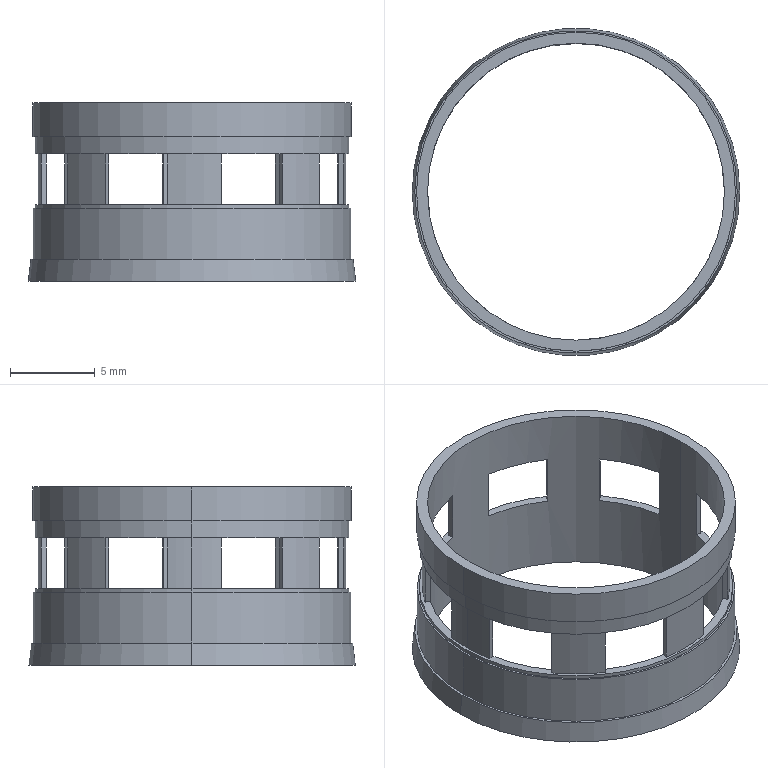Part | SolidWorks | features ICE 7, Blend 1, CirPattern 1 | 1 solid | 44 faces | box 19.3 x 19.3 x 10.5 mm | volume 297.419 mm3 | plane 23 | cylinder 19 | cone 2 | commonest cylinder face diameters 18.13 x9 18.5 x4 17.5 x2 18.72 x2 18.8 x2
STEP:
#1=CARTESIAN_POINT('',(9.4,0.,10.5));
#2=VERTEX_POINT('',#1);
#3=CARTESIAN_POINT('',(-9.4,0.,10.5));
#4=VERTEX_POINT('',#3);
#5=CARTESIAN_POINT('',(0.,0.,10.5));
#6=DIRECTION('',(0.,0.,1.));
#7=DIRECTION('',(1.,0.,0.));
#8=AXIS2_PLACEMENT_3D('',#5,#6,#7);
#9=CIRCLE('',#8,9.4);
#10=EDGE_CURVE('',#2,#4,#9,.T.);
#11=ORIENTED_EDGE('',*,*,#10,.F.);
#12=CARTESIAN_POINT('',(9.4,0.,8.5));
#13=VERTEX_POINT('',#12);
#14=CARTESIAN_POINT('',(9.4,0.,10.5));
#15=DIRECTION('',(0.,0.,-1.));
#16=VECTOR('',#15,1000.);
#17=LINE('',#14,#16);
#18=EDGE_CURVE('',#2,#13,#17,.T.);
#19=ORIENTED_EDGE('',*,*,#18,.T.);
#20=CARTESIAN_POINT('',(-9.4,0.,8.5));
#21=VERTEX_POINT('',#20);
#22=CARTESIAN_POINT('',(0.,0.,8.5));
#23=DIRECTION('',(0.,0.,1.));
#24=DIRECTION('',(1.,0.,0.));
#25=AXIS2_PLACEMENT_3D('',#22,#23,#24);
#26=CIRCLE('',#25,9.4);
#27=EDGE_CURVE('',#13,#21,#26,.T.);
#28=ORIENTED_EDGE('',*,*,#27,.T.);
#29=CARTESIAN_POINT('',(-9.4,0.,10.5));
#30=DIRECTION('',(0.,0.,-1.));
#31=VECTOR('',#30,1000.);
#32=LINE('',#29,#31);
#33=EDGE_CURVE('',#4,#21,#32,.T.);
#34=ORIENTED_EDGE('',*,*,#33,.F.);
#35=EDGE_LOOP('',(#11,#19,#28,#34));
#36=FACE_OUTER_BOUND('',#35,.T.);
#37=CARTESIAN_POINT('',(0.,0.,10.5));
#38=DIRECTION('',(0.,0.,-1.));
#39=DIRECTION('',(-1.,0.,0.));
#40=AXIS2_PLACEMENT_3D('',#37,#38,#39);
#41=CYLINDRICAL_SURFACE('',#40,9.4);
#42=ADVANCED_FACE('',(#36),#41,.T.);
#43=CARTESIAN_POINT('',(9.25,0.,8.5));
#44=VERTEX_POINT('',#43);
#45=CARTESIAN_POINT('',(-9.25,0.,8.5));
#46=VERTEX_POINT('',#45);
#47=CARTESIAN_POINT('',(0.,0.,8.5));
#48=DIRECTION('',(0.,0.,1.));
#49=DIRECTION('',(1.,0.,0.));
#50=AXIS2_PLACEMENT_3D('',#47,#48,#49);
#51=CIRCLE('',#50,9.25);
#52=EDGE_CURVE('',#44,#46,#51,.T.);
#53=ORIENTED_EDGE('',*,*,#52,.F.);
#54=CARTESIAN_POINT('',(9.25,0.,7.5));
#55=VERTEX_POINT('',#54);
#56=CARTESIAN_POINT('',(9.25,0.,8.5));
#57=DIRECTION('',(0.,0.,-1.));
#58=VECTOR('',#57,1000.);
#59=LINE('',#56,#58);
#60=EDGE_CURVE('',#44,#55,#59,.T.);
#61=ORIENTED_EDGE('',*,*,#60,.T.);
#62=CARTESIAN_POINT('',(-9.25,0.,7.5));
#63=VERTEX_POINT('',#62);
#64=CARTESIAN_POINT('',(0.,0.,7.5));
#65=DIRECTION('',(0.,0.,1.));
#66=DIRECTION('',(1.,0.,0.));
#67=AXIS2_PLACEMENT_3D('',#64,#65,#66);
#68=CIRCLE('',#67,9.25);
#69=EDGE_CURVE('',#55,#63,#68,.T.);
#70=ORIENTED_EDGE('',*,*,#69,.T.);
#71=CARTESIAN_POINT('',(-9.25,0.,8.5));
#72=DIRECTION('',(0.,0.,-1.));
#73=VECTOR('',#72,1000.);
#74=LINE('',#71,#73);
#75=EDGE_CURVE('',#46,#63,#74,.T.);
#76=ORIENTED_EDGE('',*,*,#75,.F.);
#77=EDGE_LOOP('',(#53,#61,#70,#76));
#78=FACE_OUTER_BOUND('',#77,.T.);
#79=CARTESIAN_POINT('',(0.,0.,8.5));
#80=DIRECTION('',(0.,0.,-1.));
#81=DIRECTION('',(-1.,0.,0.));
#82=AXIS2_PLACEMENT_3D('',#79,#80,#81);
#83=CYLINDRICAL_SURFACE('',#82,9.25);
#84=ADVANCED_FACE('',(#78),#83,.T.);
#85=CARTESIAN_POINT('',(-9.065,0.,7.5));
#86=VERTEX_POINT('',#85);
#87=CARTESIAN_POINT('',(-8.899,-1.727,7.5));
#88=VERTEX_POINT('',#87);
#89=CARTESIAN_POINT('',(0.,0.,7.5));
#90=DIRECTION('',(0.,0.,1.));
#91=DIRECTION('',(0.,1.,0.));
#92=AXIS2_PLACEMENT_3D('',#89,#90,#91);
#93=CIRCLE('',#92,9.065);
#94=EDGE_CURVE('',#86,#88,#93,.T.);
#95=ORIENTED_EDGE('',*,*,#94,.F.);
#96=CARTESIAN_POINT('',(-9.065,0.,4.5));
#97=VERTEX_POINT('',#96);
#98=CARTESIAN_POINT('',(-9.065,0.,7.5));
#99=DIRECTION('',(0.,0.,-1.));
#100=VECTOR('',#99,1000.);
#101=LINE('',#98,#100);
#102=EDGE_CURVE('',#86,#97,#101,.T.);
#103=ORIENTED_EDGE('',*,*,#102,.T.);
#104=CARTESIAN_POINT('',(-8.899,-1.727,4.5));
#105=VERTEX_POINT('',#104);
#106=CARTESIAN_POINT('',(0.,0.,4.5));
#107=DIRECTION('',(0.,0.,1.));
#108=DIRECTION('',(0.,1.,0.));
#109=AXIS2_PLACEMENT_3D('',#106,#107,#108);
#110=CIRCLE('',#109,9.065);
#111=EDGE_CURVE('',#97,#105,#110,.T.);
#112=ORIENTED_EDGE('',*,*,#111,.T.);
#113=CARTESIAN_POINT('',(-8.899,-1.727,7.5));
#114=DIRECTION('',(0.,0.,-1.));
#115=VECTOR('',#114,1000.);
#116=LINE('',#113,#115);
#117=EDGE_CURVE('',#88,#105,#116,.T.);
#118=ORIENTED_EDGE('',*,*,#117,.F.);
#119=EDGE_LOOP('',(#95,#103,#112,#118));
#120=FACE_OUTER_BOUND('',#119,.T.);
#121=CARTESIAN_POINT('',(0.,0.,7.5));
#122=DIRECTION('',(0.,0.,-1.));
#123=DIRECTION('',(-1.,0.,0.));
#124=AXIS2_PLACEMENT_3D('',#121,#122,#123);
#125=CYLINDRICAL_SURFACE('',#124,9.065);
#126=ADVANCED_FACE('',(#120),#125,.T.);
#127=CARTESIAN_POINT('',(7.253,-4.895,7.5));
#128=VERTEX_POINT('',#127);
#129=CARTESIAN_POINT('',(8.642,-1.372,7.5));
#130=VERTEX_POINT('',#129);
#131=CARTESIAN_POINT('',(0.,0.,7.5));
#132=DIRECTION('',(0.,0.,1.));
#133=DIRECTION('',(1.,0.,0.));
#134=AXIS2_PLACEMENT_3D('',#131,#132,#133);
#135=CIRCLE('',#134,8.75);
#136=EDGE_CURVE('',#128,#130,#135,.T.);
#137=ORIENTED_EDGE('',*,*,#136,.F.);
#138=CARTESIAN_POINT('',(7.253,-4.895,4.5));
#139=VERTEX_POINT('',#138);
#140=CARTESIAN_POINT('',(7.253,-4.895,7.5));
#141=DIRECTION('',(0.,0.,-1.));
#142=VECTOR('',#141,1000.);
#143=LINE('',#140,#142);
#144=EDGE_CURVE('',#128,#139,#143,.T.);
#145=ORIENTED_EDGE('',*,*,#144,.T.);
#146=CARTESIAN_POINT('',(8.642,-1.372,4.5));
#147=VERTEX_POINT('',#146);
#148=CARTESIAN_POINT('',(0.,0.,4.5));
#149=DIRECTION('',(0.,0.,1.));
#150=DIRECTION('',(1.,0.,0.));
#151=AXIS2_PLACEMENT_3D('',#148,#149,#150);
#152=CIRCLE('',#151,8.75);
#153=EDGE_CURVE('',#139,#147,#152,.T.);
#154=ORIENTED_EDGE('',*,*,#153,.T.);
#155=CARTESIAN_POINT('',(8.642,-1.372,7.5));
#156=DIRECTION('',(0.,0.,-1.));
#157=VECTOR('',#156,1000.);
#158=LINE('',#155,#157);
#159=EDGE_CURVE('',#130,#147,#158,.T.);
#160=ORIENTED_EDGE('',*,*,#159,.F.);
#161=EDGE_LOOP('',(#137,#145,#154,#160));
#162=FACE_BOUND('',#161,.T.);
#163=CARTESIAN_POINT('',(5.141,-7.081,7.5));
#164=VERTEX_POINT('',#163);
#165=CARTESIAN_POINT('',(5.141,-7.081,4.5));
#166=VERTEX_POINT('',#165);
#167=CARTESIAN_POINT('',(5.141,-7.081,7.5));
#168=DIRECTION('',(0.,0.,-1.));
#169=VECTOR('',#168,1000.);
#170=LINE('',#167,#169);
#171=EDGE_CURVE('',#164,#166,#170,.T.);
#172=ORIENTED_EDGE('',*,*,#171,.F.);
#173=CARTESIAN_POINT('',(1.667,-8.59,7.5));
#174=VERTEX_POINT('',#173);
#175=CARTESIAN_POINT('',(0.,0.,7.5));
#176=DIRECTION('',(0.,0.,1.));
#177=DIRECTION('',(1.,0.,0.));
#178=AXIS2_PLACEMENT_3D('',#175,#176,#177);
#179=CIRCLE('',#178,8.75);
#180=EDGE_CURVE('',#174,#164,#179,.T.);
#181=ORIENTED_EDGE('',*,*,#180,.F.);
#182=CARTESIAN_POINT('',(1.667,-8.59,4.5));
#183=VERTEX_POINT('',#182);
#184=CARTESIAN_POINT('',(1.667,-8.59,7.5));
#185=DIRECTION('',(0.,0.,-1.));
#186=VECTOR('',#185,1000.);
#187=LINE('',#184,#186);
#188=EDGE_CURVE('',#174,#183,#187,.T.);
#189=ORIENTED_EDGE('',*,*,#188,.T.);
#190=CARTESIAN_POINT('',(0.,0.,4.5));
#191=DIRECTION('',(0.,0.,1.));
#192=DIRECTION('',(1.,0.,0.));
#193=AXIS2_PLACEMENT_3D('',#190,#191,#192);
#194=CIRCLE('',#193,8.75);
#195=EDGE_CURVE('',#183,#166,#194,.T.);
#196=ORIENTED_EDGE('',*,*,#195,.T.);
#197=EDGE_LOOP('',(#172,#181,#189,#196));
#198=FACE_BOUND('',#197,.T.);
#199=CARTESIAN_POINT('',(-1.372,-8.642,7.5));
#200=VERTEX_POINT('',#199);
#201=CARTESIAN_POINT('',(-1.372,-8.642,4.5));
#202=VERTEX_POINT('',#201);
#203=CARTESIAN_POINT('',(-1.372,-8.642,7.5));
#204=DIRECTION('',(0.,0.,-1.));
#205=VECTOR('',#204,1000.);
#206=LINE('',#203,#205);
#207=EDGE_CURVE('',#200,#202,#206,.T.);
#208=ORIENTED_EDGE('',*,*,#207,.F.);
#209=CARTESIAN_POINT('',(-4.895,-7.253,7.5));
#210=VERTEX_POINT('',#209);
#211=CARTESIAN_POINT('',(0.,0.,7.5));
#212=DIRECTION('',(0.,0.,1.));
#213=DIRECTION('',(1.,0.,0.));
#214=AXIS2_PLACEMENT_3D('',#211,#212,#213);
#215=CIRCLE('',#214,8.75);
#216=EDGE_CURVE('',#210,#200,#215,.T.);
#217=ORIENTED_EDGE('',*,*,#216,.F.);
#218=CARTESIAN_POINT('',(-4.895,-7.253,4.5));
#219=VERTEX_POINT('',#218);
#220=CARTESIAN_POINT('',(-4.895,-7.253,7.5));
#221=DIRECTION('',(0.,0.,-1.));
#222=VECTOR('',#221,1000.);
#223=LINE('',#220,#222);
#224=EDGE_CURVE('',#210,#219,#223,.T.);
#225=ORIENTED_EDGE('',*,*,#224,.T.);
#226=CARTESIAN_POINT('',(0.,0.,4.5));
#227=DIRECTION('',(0.,0.,1.));
#228=DIRECTION('',(1.,0.,0.));
#229=AXIS2_PLACEMENT_3D('',#226,#227,#228);
#230=CIRCLE('',#229,8.75);
#231=EDGE_CURVE('',#219,#202,#230,.T.);
#232=ORIENTED_EDGE('',*,*,#231,.T.);
#233=EDGE_LOOP('',(#208,#217,#225,#232));
#234=FACE_BOUND('',#233,.T.);
#235=CARTESIAN_POINT('',(-7.081,-5.141,7.5));
#236=VERTEX_POINT('',#235);
#237=CARTESIAN_POINT('',(-7.081,-5.141,4.5));
#238=VERTEX_POINT('',#237);
#239=CARTESIAN_POINT('',(-7.081,-5.141,7.5));
#240=DIRECTION('',(0.,0.,-1.));
#241=VECTOR('',#240,1000.);
#242=LINE('',#239,#241);
#243=EDGE_CURVE('',#236,#238,#242,.T.);
#244=ORIENTED_EDGE('',*,*,#243,.F.);
#245=CARTESIAN_POINT('',(-8.59,-1.667,7.5));
#246=VERTEX_POINT('',#245);
#247=CARTESIAN_POINT('',(0.,0.,7.5));
#248=DIRECTION('',(0.,0.,1.));
#249=DIRECTION('',(1.,0.,0.));
#250=AXIS2_PLACEMENT_3D('',#247,#248,#249);
#251=CIRCLE('',#250,8.75);
#252=EDGE_CURVE('',#246,#236,#251,.T.);
#253=ORIENTED_EDGE('',*,*,#252,.F.);
#254=CARTESIAN_POINT('',(-8.59,-1.667,4.5));
#255=VERTEX_POINT('',#254);
#256=CARTESIAN_POINT('',(-8.59,-1.667,7.5));
#257=DIRECTION('',(0.,0.,-1.));
#258=VECTOR('',#257,1000.);
#259=LINE('',#256,#258);
#260=EDGE_CURVE('',#246,#255,#259,.T.);
#261=ORIENTED_EDGE('',*,*,#260,.T.);
#262=CARTESIAN_POINT('',(0.,0.,4.5));
#263=DIRECTION('',(0.,0.,1.));
#264=DIRECTION('',(1.,0.,0.));
#265=AXIS2_PLACEMENT_3D('',#262,#263,#264);
#266=CIRCLE('',#265,8.75);
#267=EDGE_CURVE('',#255,#238,#266,.T.);
#268=ORIENTED_EDGE('',*,*,#267,.T.);
#269=EDGE_LOOP('',(#244,#253,#261,#268));
#270=FACE_BOUND('',#269,.T.);
#271=CARTESIAN_POINT('',(-8.75,0.,0.));
#272=VERTEX_POINT('',#271);
#273=CARTESIAN_POINT('',(8.75,0.,0.));
#274=VERTEX_POINT('',#273);
#275=CARTESIAN_POINT('',(0.,0.,0.));
#276=DIRECTION('',(0.,0.,1.));
#277=DIRECTION('',(1.,0.,0.));
#278=AXIS2_PLACEMENT_3D('',#275,#276,#277);
#279=CIRCLE('',#278,8.75);
#280=EDGE_CURVE('',#272,#274,#279,.T.);
#281=ORIENTED_EDGE('',*,*,#280,.F.);
#282=CARTESIAN_POINT('',(-8.75,0.,10.5));
#283=VERTEX_POINT('',#282);
#284=CARTESIAN_POINT('',(-8.75,0.,-5.7));
#285=DIRECTION('',(0.,0.,1.));
#286=VECTOR('',#285,1000.);
#287=LINE('',#284,#286);
#288=EDGE_CURVE('',#272,#283,#287,.T.);
#289=ORIENTED_EDGE('',*,*,#288,.T.);
#290=CARTESIAN_POINT('',(8.75,0.,10.5));
#291=VERTEX_POINT('',#290);
#292=CARTESIAN_POINT('',(0.,0.,10.5));
#293=DIRECTION('',(0.,0.,1.));
#294=DIRECTION('',(1.,0.,0.));
#295=AXIS2_PLACEMENT_3D('',#292,#293,#294);
#296=CIRCLE('',#295,8.75);
#297=EDGE_CURVE('',#283,#291,#296,.T.);
#298=ORIENTED_EDGE('',*,*,#297,.T.);
#299=CARTESIAN_POINT('',(8.75,0.,-5.7));
#300=DIRECTION('',(0.,0.,1.));
#301=VECTOR('',#300,1000.);
#302=LINE('',#299,#301);
#303=EDGE_CURVE('',#274,#291,#302,.T.);
#304=ORIENTED_EDGE('',*,*,#303,.F.);
#305=EDGE_LOOP('',(#281,#289,#298,#304));
#306=FACE_OUTER_BOUND('',#305,.T.);
#307=CARTESIAN_POINT('',(0.,0.,-5.7));
#308=DIRECTION('',(0.,0.,1.));
#309=DIRECTION('',(1.,0.,0.));
#310=AXIS2_PLACEMENT_3D('',#307,#308,#309);
#311=CYLINDRICAL_SURFACE('',#310,8.75);
#312=ADVANCED_FACE('',(#162,#198,#234,#270,#306),#311,.F.);
#313=CARTESIAN_POINT('',(9.25,0.,4.5));
#314=VERTEX_POINT('',#313);
#315=CARTESIAN_POINT('',(-9.25,0.,4.5));
#316=VERTEX_POINT('',#315);
#317=CARTESIAN_POINT('',(0.,0.,4.5));
#318=DIRECTION('',(0.,0.,1.));
#319=DIRECTION('',(1.,0.,0.));
#320=AXIS2_PLACEMENT_3D('',#317,#318,#319);
#321=CIRCLE('',#320,9.25);
#322=EDGE_CURVE('',#314,#316,#321,.T.);
#323=ORIENTED_EDGE('',*,*,#322,.F.);
#324=CARTESIAN_POINT('',(9.25,0.,4.3));
#325=VERTEX_POINT('',#324);
#326=CARTESIAN_POINT('',(9.25,0.,4.5));
#327=DIRECTION('',(0.,0.,-1.));
#328=VECTOR('',#327,1000.);
#329=LINE('',#326,#328);
#330=EDGE_CURVE('',#314,#325,#329,.T.);
#331=ORIENTED_EDGE('',*,*,#330,.T.);
#332=CARTESIAN_POINT('',(-9.25,0.,4.3));
#333=VERTEX_POINT('',#332);
#334=CARTESIAN_POINT('',(0.,0.,4.3));
#335=DIRECTION('',(0.,0.,1.));
#336=DIRECTION('',(1.,0.,0.));
#337=AXIS2_PLACEMENT_3D('',#334,#335,#336);
#338=CIRCLE('',#337,9.25);
#339=EDGE_CURVE('',#325,#333,#338,.T.);
#340=ORIENTED_EDGE('',*,*,#339,.T.);
#341=CARTESIAN_POINT('',(-9.25,0.,4.5));
#342=DIRECTION('',(0.,0.,-1.));
#343=VECTOR('',#342,1000.);
#344=LINE('',#341,#343);
#345=EDGE_CURVE('',#316,#333,#344,.T.);
#346=ORIENTED_EDGE('',*,*,#345,.F.);
#347=EDGE_LOOP('',(#323,#331,#340,#346));
#348=FACE_OUTER_BOUND('',#347,.T.);
#349=CARTESIAN_POINT('',(0.,0.,4.5));
#350=DIRECTION('',(0.,0.,-1.));
#351=DIRECTION('',(-1.,0.,0.));
#352=AXIS2_PLACEMENT_3D('',#349,#350,#351);
#353=CYLINDRICAL_SURFACE('',#352,9.25);
#354=ADVANCED_FACE('',(#348),#353,.T.);
#355=CARTESIAN_POINT('',(9.36,0.,4.3));
#356=VERTEX_POINT('',#355);
#357=CARTESIAN_POINT('',(-9.36,0.,4.3));
#358=VERTEX_POINT('',#357);
#359=CARTESIAN_POINT('',(0.,0.,4.3));
#360=DIRECTION('',(0.,0.,1.));
#361=DIRECTION('',(1.,0.,0.));
#362=AXIS2_PLACEMENT_3D('',#359,#360,#361);
#363=CIRCLE('',#362,9.36);
#364=EDGE_CURVE('',#356,#358,#363,.T.);
#365=ORIENTED_EDGE('',*,*,#364,.F.);
#366=CARTESIAN_POINT('',(9.36,0.,1.3));
#367=VERTEX_POINT('',#366);
#368=CARTESIAN_POINT('',(9.36,0.,4.3));
#369=DIRECTION('',(0.,0.,-1.));
#370=VECTOR('',#369,1000.);
#371=LINE('',#368,#370);
#372=EDGE_CURVE('',#356,#367,#371,.T.);
#373=ORIENTED_EDGE('',*,*,#372,.T.);
#374=CARTESIAN_POINT('',(-9.36,0.,1.3));
#375=VERTEX_POINT('',#374);
#376=CARTESIAN_POINT('',(0.,0.,1.3));
#377=DIRECTION('',(0.,0.,1.));
#378=DIRECTION('',(1.,0.,0.));
#379=AXIS2_PLACEMENT_3D('',#376,#377,#378);
#380=CIRCLE('',#379,9.36);
#381=EDGE_CURVE('',#367,#375,#380,.T.);
#382=ORIENTED_EDGE('',*,*,#381,.T.);
#383=CARTESIAN_POINT('',(-9.36,0.,4.3));
#384=DIRECTION('',(0.,0.,-1.));
#385=VECTOR('',#384,1000.);
#386=LINE('',#383,#385);
#387=EDGE_CURVE('',#358,#375,#386,.T.);
#388=ORIENTED_EDGE('',*,*,#387,.F.);
#389=EDGE_LOOP('',(#365,#373,#382,#388));
#390=FACE_OUTER_BOUND('',#389,.T.);
#391=CARTESIAN_POINT('',(0.,0.,4.3));
#392=DIRECTION('',(0.,0.,-1.));
#393=DIRECTION('',(-1.,0.,0.));
#394=AXIS2_PLACEMENT_3D('',#391,#392,#393);
#395=CYLINDRICAL_SURFACE('',#394,9.36);
#396=ADVANCED_FACE('',(#390),#395,.T.);
#397=CARTESIAN_POINT('',(9.5,0.,1.3));
#398=VERTEX_POINT('',#397);
#399=CARTESIAN_POINT('',(-9.5,0.,1.3));
#400=VERTEX_POINT('',#399);
#401=CARTESIAN_POINT('',(0.,0.,1.3));
#402=DIRECTION('',(0.,0.,1.));
#403=DIRECTION('',(1.,0.,0.));
#404=AXIS2_PLACEMENT_3D('',#401,#402,#403);
#405=CIRCLE('',#404,9.5);
#406=EDGE_CURVE('',#398,#400,#405,.T.);
#407=ORIENTED_EDGE('',*,*,#406,.F.);
#408=CARTESIAN_POINT('',(9.65,0.,0.));
#409=VERTEX_POINT('',#408);
#410=CARTESIAN_POINT('',(9.5,0.,1.3));
#411=DIRECTION('',(0.1146,0.,-0.9934));
#412=VECTOR('',#411,1000.);
#413=LINE('',#410,#412);
#414=EDGE_CURVE('',#398,#409,#413,.T.);
#415=ORIENTED_EDGE('',*,*,#414,.T.);
#416=CARTESIAN_POINT('',(-9.65,0.,0.));
#417=VERTEX_POINT('',#416);
#418=CARTESIAN_POINT('',(0.,0.,0.));
#419=DIRECTION('',(0.,0.,1.));
#420=DIRECTION('',(1.,0.,0.));
#421=AXIS2_PLACEMENT_3D('',#418,#419,#420);
#422=CIRCLE('',#421,9.65);
#423=EDGE_CURVE('',#409,#417,#422,.T.);
#424=ORIENTED_EDGE('',*,*,#423,.T.);
#425=CARTESIAN_POINT('',(-9.5,0.,1.3));
#426=DIRECTION('',(-0.1146,0.,-0.9934));
#427=VECTOR('',#426,1000.);
#428=LINE('',#425,#427);
#429=EDGE_CURVE('',#400,#417,#428,.T.);
#430=ORIENTED_EDGE('',*,*,#429,.F.);
#431=EDGE_LOOP('',(#407,#415,#424,#430));
#432=FACE_OUTER_BOUND('',#431,.T.);
#433=CARTESIAN_POINT('',(0.,0.,1.3));
#434=DIRECTION('',(0.,0.,-1.));
#435=DIRECTION('',(-1.,0.,0.));
#436=AXIS2_PLACEMENT_3D('',#433,#434,#435);
#437=CONICAL_SURFACE('',#436,9.5,0.1149);
#438=ADVANCED_FACE('',(#432),#437,.T.);
#439=CARTESIAN_POINT('',(0.,0.,4.5));
#440=DIRECTION('',(0.,0.,1.));
#441=DIRECTION('',(1.,0.,0.));
#442=AXIS2_PLACEMENT_3D('',#439,#440,#441);
#443=CIRCLE('',#442,9.25);
#444=EDGE_CURVE('',#316,#314,#443,.T.);
#445=ORIENTED_EDGE('',*,*,#444,.T.);
#446=ORIENTED_EDGE('',*,*,#322,.T.);
#447=EDGE_LOOP('',(#445,#446));
#448=FACE_OUTER_BOUND('',#447,.T.);
#449=CARTESIAN_POINT('',(4.895,7.253,4.5));
#450=VERTEX_POINT('',#449);
#451=CARTESIAN_POINT('',(1.372,8.642,4.5));
#452=VERTEX_POINT('',#451);
#453=CARTESIAN_POINT('',(0.,0.,4.5));
#454=DIRECTION('',(0.,0.,1.));
#455=DIRECTION('',(1.,0.,0.));
#456=AXIS2_PLACEMENT_3D('',#453,#454,#455);
#457=CIRCLE('',#456,8.75);
#458=EDGE_CURVE('',#450,#452,#457,.T.);
#459=ORIENTED_EDGE('',*,*,#458,.F.);
#460=CARTESIAN_POINT('',(5.071,7.513,4.5));
#461=VERTEX_POINT('',#460);
#462=CARTESIAN_POINT('',(4.895,7.253,4.5));
#463=DIRECTION('',(-0.5595,-0.8289,0.));
#464=VECTOR('',#463,1000.);
#465=LINE('',#462,#464);
#466=EDGE_CURVE('',#461,#450,#465,.T.);
#467=ORIENTED_EDGE('',*,*,#466,.F.);
#468=CARTESIAN_POINT('',(7.335,5.326,4.5));
#469=VERTEX_POINT('',#468);
#470=CARTESIAN_POINT('',(0.,0.,4.5));
#471=DIRECTION('',(0.,0.,1.));
#472=DIRECTION('',(0.7071,-0.7071,0.));
#473=AXIS2_PLACEMENT_3D('',#470,#471,#472);
#474=CIRCLE('',#473,9.065);
#475=EDGE_CURVE('',#469,#461,#474,.T.);
#476=ORIENTED_EDGE('',*,*,#475,.F.);
#477=CARTESIAN_POINT('',(7.081,5.141,4.5));
#478=VERTEX_POINT('',#477);
#479=CARTESIAN_POINT('',(7.081,5.141,4.5));
#480=DIRECTION('',(0.8092,0.5875,0.));
#481=VECTOR('',#480,1000.);
#482=LINE('',#479,#481);
#483=EDGE_CURVE('',#478,#469,#482,.T.);
#484=ORIENTED_EDGE('',*,*,#483,.F.);
#485=CARTESIAN_POINT('',(8.59,1.667,4.5));
#486=VERTEX_POINT('',#485);
#487=CARTESIAN_POINT('',(0.,0.,4.5));
#488=DIRECTION('',(0.,0.,1.));
#489=DIRECTION('',(1.,0.,0.));
#490=AXIS2_PLACEMENT_3D('',#487,#488,#489);
#491=CIRCLE('',#490,8.75);
#492=EDGE_CURVE('',#486,#478,#491,.T.);
#493=ORIENTED_EDGE('',*,*,#492,.F.);
#494=CARTESIAN_POINT('',(8.899,1.727,4.5));
#495=VERTEX_POINT('',#494);
#496=CARTESIAN_POINT('',(8.59,1.667,4.5));
#497=DIRECTION('',(-0.9817,-0.1905,0.));
#498=VECTOR('',#497,1000.);
#499=LINE('',#496,#498);
#500=EDGE_CURVE('',#495,#486,#499,.T.);
#501=ORIENTED_EDGE('',*,*,#500,.F.);
#502=CARTESIAN_POINT('',(8.953,-1.421,4.5));
#503=VERTEX_POINT('',#502);
#504=CARTESIAN_POINT('',(0.,0.,4.5));
#505=DIRECTION('',(0.,0.,1.));
#506=DIRECTION('',(0.,-1.,0.));
#507=AXIS2_PLACEMENT_3D('',#504,#505,#506);
#508=CIRCLE('',#507,9.065);
#509=EDGE_CURVE('',#503,#495,#508,.T.);
#510=ORIENTED_EDGE('',*,*,#509,.F.);
#511=CARTESIAN_POINT('',(8.642,-1.372,4.5));
#512=DIRECTION('',(0.9876,-0.1568,0.));
#513=VECTOR('',#512,1000.);
#514=LINE('',#511,#513);
#515=EDGE_CURVE('',#147,#503,#514,.T.);
#516=ORIENTED_EDGE('',*,*,#515,.F.);
#517=ORIENTED_EDGE('',*,*,#153,.F.);
#518=CARTESIAN_POINT('',(7.513,-5.071,4.5));
#519=VERTEX_POINT('',#518);
#520=CARTESIAN_POINT('',(7.253,-4.895,4.5));
#521=DIRECTION('',(-0.8289,0.5595,0.));
#522=VECTOR('',#521,1000.);
#523=LINE('',#520,#522);
#524=EDGE_CURVE('',#519,#139,#523,.T.);
#525=ORIENTED_EDGE('',*,*,#524,.F.);
#526=CARTESIAN_POINT('',(5.326,-7.335,4.5));
#527=VERTEX_POINT('',#526);
#528=CARTESIAN_POINT('',(0.,0.,4.5));
#529=DIRECTION('',(0.,0.,1.));
#530=DIRECTION('',(-0.7071,-0.7071,0.));
#531=AXIS2_PLACEMENT_3D('',#528,#529,#530);
#532=CIRCLE('',#531,9.065);
#533=EDGE_CURVE('',#527,#519,#532,.T.);
#534=ORIENTED_EDGE('',*,*,#533,.F.);
#535=CARTESIAN_POINT('',(5.141,-7.081,4.5));
#536=DIRECTION('',(0.5875,-0.8092,0.));
#537=VECTOR('',#536,1000.);
#538=LINE('',#535,#537);
#539=EDGE_CURVE('',#166,#527,#538,.T.);
#540=ORIENTED_EDGE('',*,*,#539,.F.);
#541=ORIENTED_EDGE('',*,*,#195,.F.);
#542=CARTESIAN_POINT('',(1.727,-8.899,4.5));
#543=VERTEX_POINT('',#542);
#544=CARTESIAN_POINT('',(1.667,-8.59,4.5));
#545=DIRECTION('',(-0.1905,0.9817,0.));
#546=VECTOR('',#545,1000.);
#547=LINE('',#544,#546);
#548=EDGE_CURVE('',#543,#183,#547,.T.);
#549=ORIENTED_EDGE('',*,*,#548,.F.);
#550=CARTESIAN_POINT('',(-1.421,-8.953,4.5));
#551=VERTEX_POINT('',#550);
#552=CARTESIAN_POINT('',(0.,0.,4.5));
#553=DIRECTION('',(0.,0.,1.));
#554=DIRECTION('',(-1.,0.,0.));
#555=AXIS2_PLACEMENT_3D('',#552,#553,#554);
#556=CIRCLE('',#555,9.065);
#557=EDGE_CURVE('',#551,#543,#556,.T.);
#558=ORIENTED_EDGE('',*,*,#557,.F.);
#559=CARTESIAN_POINT('',(-1.372,-8.642,4.5));
#560=DIRECTION('',(-0.1568,-0.9876,0.));
#561=VECTOR('',#560,1000.);
#562=LINE('',#559,#561);
#563=EDGE_CURVE('',#202,#551,#562,.T.);
#564=ORIENTED_EDGE('',*,*,#563,.F.);
#565=ORIENTED_EDGE('',*,*,#231,.F.);
#566=CARTESIAN_POINT('',(-5.071,-7.513,4.5));
#567=VERTEX_POINT('',#566);
#568=CARTESIAN_POINT('',(-4.895,-7.253,4.5));
#569=DIRECTION('',(0.5595,0.8289,0.));
#570=VECTOR('',#569,1000.);
#571=LINE('',#568,#570);
#572=EDGE_CURVE('',#567,#219,#571,.T.);
#573=ORIENTED_EDGE('',*,*,#572,.F.);
#574=CARTESIAN_POINT('',(-7.335,-5.326,4.5));
#575=VERTEX_POINT('',#574);
#576=CARTESIAN_POINT('',(0.,0.,4.5));
#577=DIRECTION('',(0.,0.,1.));
#578=DIRECTION('',(-0.7071,0.7071,0.));
#579=AXIS2_PLACEMENT_3D('',#576,#577,#578);
#580=CIRCLE('',#579,9.065);
#581=EDGE_CURVE('',#575,#567,#580,.T.);
#582=ORIENTED_EDGE('',*,*,#581,.F.);
#583=CARTESIAN_POINT('',(-7.081,-5.141,4.5));
#584=DIRECTION('',(-0.8092,-0.5875,0.));
#585=VECTOR('',#584,1000.);
#586=LINE('',#583,#585);
#587=EDGE_CURVE('',#238,#575,#586,.T.);
#588=ORIENTED_EDGE('',*,*,#587,.F.);
#589=ORIENTED_EDGE('',*,*,#267,.F.);
#590=CARTESIAN_POINT('',(-8.59,-1.667,4.5));
#591=DIRECTION('',(0.9817,0.1905,0.));
#592=VECTOR('',#591,1000.);
#593=LINE('',#590,#592);
#594=EDGE_CURVE('',#105,#255,#593,.T.);
#595=ORIENTED_EDGE('',*,*,#594,.F.);
#596=ORIENTED_EDGE('',*,*,#111,.F.);
#597=CARTESIAN_POINT('',(-8.953,1.421,4.5));
#598=VERTEX_POINT('',#597);
#599=CARTESIAN_POINT('',(0.,0.,4.5));
#600=DIRECTION('',(0.,0.,1.));
#601=DIRECTION('',(0.,1.,0.));
#602=AXIS2_PLACEMENT_3D('',#599,#600,#601);
#603=CIRCLE('',#602,9.065);
#604=EDGE_CURVE('',#598,#97,#603,.T.);
#605=ORIENTED_EDGE('',*,*,#604,.F.);
#606=CARTESIAN_POINT('',(-8.642,1.372,4.5));
#607=VERTEX_POINT('',#606);
#608=CARTESIAN_POINT('',(-8.642,1.372,4.5));
#609=DIRECTION('',(-0.9876,0.1568,0.));
#610=VECTOR('',#609,1000.);
#611=LINE('',#608,#610);
#612=EDGE_CURVE('',#607,#598,#611,.T.);
#613=ORIENTED_EDGE('',*,*,#612,.F.);
#614=CARTESIAN_POINT('',(-7.253,4.895,4.5));
#615=VERTEX_POINT('',#614);
#616=CARTESIAN_POINT('',(0.,0.,4.5));
#617=DIRECTION('',(0.,0.,1.));
#618=DIRECTION('',(1.,0.,0.));
#619=AXIS2_PLACEMENT_3D('',#616,#617,#618);
#620=CIRCLE('',#619,8.75);
#621=EDGE_CURVE('',#615,#607,#620,.T.);
#622=ORIENTED_EDGE('',*,*,#621,.F.);
#623=CARTESIAN_POINT('',(-7.513,5.071,4.5));
#624=VERTEX_POINT('',#623);
#625=CARTESIAN_POINT('',(-7.253,4.895,4.5));
#626=DIRECTION('',(0.8289,-0.5595,0.));
#627=VECTOR('',#626,1000.);
#628=LINE('',#625,#627);
#629=EDGE_CURVE('',#624,#615,#628,.T.);
#630=ORIENTED_EDGE('',*,*,#629,.F.);
#631=CARTESIAN_POINT('',(-5.326,7.335,4.5));
#632=VERTEX_POINT('',#631);
#633=CARTESIAN_POINT('',(0.,0.,4.5));
#634=DIRECTION('',(0.,0.,1.));
#635=DIRECTION('',(0.7071,0.7071,0.));
#636=AXIS2_PLACEMENT_3D('',#633,#634,#635);
#637=CIRCLE('',#636,9.065);
#638=EDGE_CURVE('',#632,#624,#637,.T.);
#639=ORIENTED_EDGE('',*,*,#638,.F.);
#640=CARTESIAN_POINT('',(-5.141,7.081,4.5));
#641=VERTEX_POINT('',#640);
#642=CARTESIAN_POINT('',(-5.141,7.081,4.5));
#643=DIRECTION('',(-0.5875,0.8092,0.));
#644=VECTOR('',#643,1000.);
#645=LINE('',#642,#644);
#646=EDGE_CURVE('',#641,#632,#645,.T.);
#647=ORIENTED_EDGE('',*,*,#646,.F.);
#648=CARTESIAN_POINT('',(-1.667,8.59,4.5));
#649=VERTEX_POINT('',#648);
#650=CARTESIAN_POINT('',(0.,0.,4.5));
#651=DIRECTION('',(0.,0.,1.));
#652=DIRECTION('',(1.,0.,0.));
#653=AXIS2_PLACEMENT_3D('',#650,#651,#652);
#654=CIRCLE('',#653,8.75);
#655=EDGE_CURVE('',#649,#641,#654,.T.);
#656=ORIENTED_EDGE('',*,*,#655,.F.);
#657=CARTESIAN_POINT('',(-1.727,8.899,4.5));
#658=VERTEX_POINT('',#657);
#659=CARTESIAN_POINT('',(-1.667,8.59,4.5));
#660=DIRECTION('',(0.1905,-0.9817,0.));
#661=VECTOR('',#660,1000.);
#662=LINE('',#659,#661);
#663=EDGE_CURVE('',#658,#649,#662,.T.);
#664=ORIENTED_EDGE('',*,*,#663,.F.);
#665=CARTESIAN_POINT('',(1.421,8.953,4.5));
#666=VERTEX_POINT('',#665);
#667=CARTESIAN_POINT('',(0.,0.,4.5));
#668=DIRECTION('',(0.,0.,1.));
#669=DIRECTION('',(1.,0.,0.));
#670=AXIS2_PLACEMENT_3D('',#667,#668,#669);
#671=CIRCLE('',#670,9.065);
#672=EDGE_CURVE('',#666,#658,#671,.T.);
#673=ORIENTED_EDGE('',*,*,#672,.F.);
#674=CARTESIAN_POINT('',(1.372,8.642,4.5));
#675=DIRECTION('',(0.1568,0.9876,0.));
#676=VECTOR('',#675,1000.);
#677=LINE('',#674,#676);
#678=EDGE_CURVE('',#452,#666,#677,.T.);
#679=ORIENTED_EDGE('',*,*,#678,.F.);
#680=EDGE_LOOP('',(#459,#467,#476,#484,#493,#501,#510,#516,#517,#525,#534,#540,#541,#549,#558,#564,#565,#573,#582,#588,#589,#595,#596,#605,#613,#622,#630,#639,#647,#656,#664,#673,#679));
#681=FACE_BOUND('',#680,.T.);
#682=CARTESIAN_POINT('',(0.,0.,4.5));
#683=DIRECTION('',(0.,0.,1.));
#684=DIRECTION('',(1.,0.,0.));
#685=AXIS2_PLACEMENT_3D('',#682,#683,#684);
#686=PLANE('',#685);
#687=ADVANCED_FACE('',(#448,#681),#686,.T.);
#688=CARTESIAN_POINT('',(0.,0.,1.3));
#689=DIRECTION('',(0.,0.,1.));
#690=DIRECTION('',(1.,0.,0.));
#691=AXIS2_PLACEMENT_3D('',#688,#689,#690);
#692=CIRCLE('',#691,9.36);
#693=EDGE_CURVE('',#375,#367,#692,.T.);
#694=ORIENTED_EDGE('',*,*,#693,.F.);
#695=ORIENTED_EDGE('',*,*,#381,.F.);
#696=EDGE_LOOP('',(#694,#695));
#697=FACE_BOUND('',#696,.T.);
#698=CARTESIAN_POINT('',(0.,0.,1.3));
#699=DIRECTION('',(0.,0.,1.));
#700=DIRECTION('',(1.,0.,0.));
#701=AXIS2_PLACEMENT_3D('',#698,#699,#700);
#702=CIRCLE('',#701,9.5);
#703=EDGE_CURVE('',#400,#398,#702,.T.);
#704=ORIENTED_EDGE('',*,*,#703,.T.);
#705=ORIENTED_EDGE('',*,*,#406,.T.);
#706=EDGE_LOOP('',(#704,#705));
#707=FACE_OUTER_BOUND('',#706,.T.);
#708=CARTESIAN_POINT('',(0.,0.,1.3));
#709=DIRECTION('',(0.,0.,1.));
#710=DIRECTION('',(1.,0.,0.));
#711=AXIS2_PLACEMENT_3D('',#708,#709,#710);
#712=PLANE('',#711);
#713=ADVANCED_FACE('',(#697,#707),#712,.T.);
#714=CARTESIAN_POINT('',(0.,0.,0.));
#715=DIRECTION('',(0.,0.,1.));
#716=DIRECTION('',(1.,0.,0.));
#717=AXIS2_PLACEMENT_3D('',#714,#715,#716);
#718=CIRCLE('',#717,8.75);
#719=EDGE_CURVE('',#274,#272,#718,.T.);
#720=ORIENTED_EDGE('',*,*,#719,.T.);
#721=ORIENTED_EDGE('',*,*,#280,.T.);
#722=EDGE_LOOP('',(#720,#721));
#723=FACE_BOUND('',#722,.T.);
#724=CARTESIAN_POINT('',(0.,0.,0.));
#725=DIRECTION('',(0.,0.,1.));
#726=DIRECTION('',(1.,0.,0.));
#727=AXIS2_PLACEMENT_3D('',#724,#725,#726);
#728=CIRCLE('',#727,9.65);
#729=EDGE_CURVE('',#417,#409,#728,.T.);
#730=ORIENTED_EDGE('',*,*,#729,.F.);
#731=ORIENTED_EDGE('',*,*,#423,.F.);
#732=EDGE_LOOP('',(#730,#731));
#733=FACE_OUTER_BOUND('',#732,.T.);
#734=CARTESIAN_POINT('',(0.,0.,0.));
#735=DIRECTION('',(0.,0.,1.));
#736=DIRECTION('',(1.,0.,0.));
#737=AXIS2_PLACEMENT_3D('',#734,#735,#736);
#738=PLANE('',#737);
#739=ADVANCED_FACE('',(#723,#733),#738,.F.);
#740=ORIENTED_EDGE('',*,*,#414,.F.);
#741=ORIENTED_EDGE('',*,*,#703,.F.);
#742=ORIENTED_EDGE('',*,*,#429,.T.);
#743=ORIENTED_EDGE('',*,*,#729,.T.);
#744=EDGE_LOOP('',(#740,#741,#742,#743));
#745=FACE_OUTER_BOUND('',#744,.T.);
#746=CARTESIAN_POINT('',(0.,0.,1.3));
#747=DIRECTION('',(0.,0.,-1.));
#748=DIRECTION('',(-1.,0.,0.));
#749=AXIS2_PLACEMENT_3D('',#746,#747,#748);
#750=CONICAL_SURFACE('',#749,9.5,0.1149);
#751=ADVANCED_FACE('',(#745),#750,.T.);
#752=ORIENTED_EDGE('',*,*,#372,.F.);
#753=CARTESIAN_POINT('',(0.,0.,4.3));
#754=DIRECTION('',(0.,0.,1.));
#755=DIRECTION('',(1.,0.,0.));
#756=AXIS2_PLACEMENT_3D('',#753,#754,#755);
#757=CIRCLE('',#756,9.36);
#758=EDGE_CURVE('',#358,#356,#757,.T.);
#759=ORIENTED_EDGE('',*,*,#758,.F.);
#760=ORIENTED_EDGE('',*,*,#387,.T.);
#761=ORIENTED_EDGE('',*,*,#693,.T.);
#762=EDGE_LOOP('',(#752,#759,#760,#761));
#763=FACE_OUTER_BOUND('',#762,.T.);
#764=CARTESIAN_POINT('',(0.,0.,4.3));
#765=DIRECTION('',(0.,0.,-1.));
#766=DIRECTION('',(-1.,0.,0.));
#767=AXIS2_PLACEMENT_3D('',#764,#765,#766);
#768=CYLINDRICAL_SURFACE('',#767,9.36);
#769=ADVANCED_FACE('',(#763),#768,.T.);
#770=CARTESIAN_POINT('',(0.,0.,4.3));
#771=DIRECTION('',(0.,0.,1.));
#772=DIRECTION('',(1.,0.,0.));
#773=AXIS2_PLACEMENT_3D('',#770,#771,#772);
#774=CIRCLE('',#773,9.25);
#775=EDGE_CURVE('',#333,#325,#774,.T.);
#776=ORIENTED_EDGE('',*,*,#775,.F.);
#777=ORIENTED_EDGE('',*,*,#339,.F.);
#778=EDGE_LOOP('',(#776,#777));
#779=FACE_BOUND('',#778,.T.);
#780=ORIENTED_EDGE('',*,*,#758,.T.);
#781=ORIENTED_EDGE('',*,*,#364,.T.);
#782=EDGE_LOOP('',(#780,#781));
#783=FACE_OUTER_BOUND('',#782,.T.);
#784=CARTESIAN_POINT('',(0.,0.,4.3));
#785=DIRECTION('',(0.,0.,1.));
#786=DIRECTION('',(1.,0.,0.));
#787=AXIS2_PLACEMENT_3D('',#784,#785,#786);
#788=PLANE('',#787);
#789=ADVANCED_FACE('',(#779,#783),#788,.T.);
#790=ORIENTED_EDGE('',*,*,#330,.F.);
#791=ORIENTED_EDGE('',*,*,#444,.F.);
#792=ORIENTED_EDGE('',*,*,#345,.T.);
#793=ORIENTED_EDGE('',*,*,#775,.T.);
#794=EDGE_LOOP('',(#790,#791,#792,#793));
#795=FACE_OUTER_BOUND('',#794,.T.);
#796=CARTESIAN_POINT('',(0.,0.,4.5));
#797=DIRECTION('',(0.,0.,-1.));
#798=DIRECTION('',(-1.,0.,0.));
#799=AXIS2_PLACEMENT_3D('',#796,#797,#798);
#800=CYLINDRICAL_SURFACE('',#799,9.25);
#801=ADVANCED_FACE('',(#795),#800,.T.);
#802=ORIENTED_EDGE('',*,*,#288,.F.);
#803=ORIENTED_EDGE('',*,*,#719,.F.);
#804=ORIENTED_EDGE('',*,*,#303,.T.);
#805=CARTESIAN_POINT('',(0.,0.,10.5));
#806=DIRECTION('',(0.,0.,1.));
#807=DIRECTION('',(1.,0.,0.));
#808=AXIS2_PLACEMENT_3D('',#805,#806,#807);
#809=CIRCLE('',#808,8.75);
#810=EDGE_CURVE('',#291,#283,#809,.T.);
#811=ORIENTED_EDGE('',*,*,#810,.T.);
#812=EDGE_LOOP('',(#802,#803,#804,#811));
#813=FACE_OUTER_BOUND('',#812,.T.);
#814=CARTESIAN_POINT('',(7.081,5.141,7.5));
#815=VERTEX_POINT('',#814);
#816=CARTESIAN_POINT('',(7.081,5.141,7.5));
#817=DIRECTION('',(0.,0.,-1.));
#818=VECTOR('',#817,1000.);
#819=LINE('',#816,#818);
#820=EDGE_CURVE('',#815,#478,#819,.T.);
#821=ORIENTED_EDGE('',*,*,#820,.F.);
#822=CARTESIAN_POINT('',(8.59,1.667,7.5));
#823=VERTEX_POINT('',#822);
#824=CARTESIAN_POINT('',(0.,0.,7.5));
#825=DIRECTION('',(0.,0.,1.));
#826=DIRECTION('',(1.,0.,0.));
#827=AXIS2_PLACEMENT_3D('',#824,#825,#826);
#828=CIRCLE('',#827,8.75);
#829=EDGE_CURVE('',#823,#815,#828,.T.);
#830=ORIENTED_EDGE('',*,*,#829,.F.);
#831=CARTESIAN_POINT('',(8.59,1.667,7.5));
#832=DIRECTION('',(0.,0.,-1.));
#833=VECTOR('',#832,1000.);
#834=LINE('',#831,#833);
#835=EDGE_CURVE('',#823,#486,#834,.T.);
#836=ORIENTED_EDGE('',*,*,#835,.T.);
#837=ORIENTED_EDGE('',*,*,#492,.T.);
#838=EDGE_LOOP('',(#821,#830,#836,#837));
#839=FACE_BOUND('',#838,.T.);
#840=CARTESIAN_POINT('',(1.372,8.642,7.5));
#841=VERTEX_POINT('',#840);
#842=CARTESIAN_POINT('',(1.372,8.642,7.5));
#843=DIRECTION('',(0.,0.,-1.));
#844=VECTOR('',#843,1000.);
#845=LINE('',#842,#844);
#846=EDGE_CURVE('',#841,#452,#845,.T.);
#847=ORIENTED_EDGE('',*,*,#846,.F.);
#848=CARTESIAN_POINT('',(4.895,7.253,7.5));
#849=VERTEX_POINT('',#848);
#850=CARTESIAN_POINT('',(0.,0.,7.5));
#851=DIRECTION('',(0.,0.,1.));
#852=DIRECTION('',(1.,0.,0.));
#853=AXIS2_PLACEMENT_3D('',#850,#851,#852);
#854=CIRCLE('',#853,8.75);
#855=EDGE_CURVE('',#849,#841,#854,.T.);
#856=ORIENTED_EDGE('',*,*,#855,.F.);
#857=CARTESIAN_POINT('',(4.895,7.253,7.5));
#858=DIRECTION('',(0.,0.,-1.));
#859=VECTOR('',#858,1000.);
#860=LINE('',#857,#859);
#861=EDGE_CURVE('',#849,#450,#860,.T.);
#862=ORIENTED_EDGE('',*,*,#861,.T.);
#863=ORIENTED_EDGE('',*,*,#458,.T.);
#864=EDGE_LOOP('',(#847,#856,#862,#863));
#865=FACE_BOUND('',#864,.T.);
#866=CARTESIAN_POINT('',(-5.141,7.081,7.5));
#867=VERTEX_POINT('',#866);
#868=CARTESIAN_POINT('',(-5.141,7.081,7.5));
#869=DIRECTION('',(0.,0.,-1.));
#870=VECTOR('',#869,1000.);
#871=LINE('',#868,#870);
#872=EDGE_CURVE('',#867,#641,#871,.T.);
#873=ORIENTED_EDGE('',*,*,#872,.F.);
#874=CARTESIAN_POINT('',(-1.667,8.59,7.5));
#875=VERTEX_POINT('',#874);
#876=CARTESIAN_POINT('',(0.,0.,7.5));
#877=DIRECTION('',(0.,0.,1.));
#878=DIRECTION('',(1.,0.,0.));
#879=AXIS2_PLACEMENT_3D('',#876,#877,#878);
#880=CIRCLE('',#879,8.75);
#881=EDGE_CURVE('',#875,#867,#880,.T.);
#882=ORIENTED_EDGE('',*,*,#881,.F.);
#883=CARTESIAN_POINT('',(-1.667,8.59,7.5));
#884=DIRECTION('',(0.,0.,-1.));
#885=VECTOR('',#884,1000.);
#886=LINE('',#883,#885);
#887=EDGE_CURVE('',#875,#649,#886,.T.);
#888=ORIENTED_EDGE('',*,*,#887,.T.);
#889=ORIENTED_EDGE('',*,*,#655,.T.);
#890=EDGE_LOOP('',(#873,#882,#888,#889));
#891=FACE_BOUND('',#890,.T.);
#892=CARTESIAN_POINT('',(-8.642,1.372,7.5));
#893=VERTEX_POINT('',#892);
#894=CARTESIAN_POINT('',(-8.642,1.372,7.5));
#895=DIRECTION('',(0.,0.,-1.));
#896=VECTOR('',#895,1000.);
#897=LINE('',#894,#896);
#898=EDGE_CURVE('',#893,#607,#897,.T.);
#899=ORIENTED_EDGE('',*,*,#898,.F.);
#900=CARTESIAN_POINT('',(-7.253,4.895,7.5));
#901=VERTEX_POINT('',#900);
#902=CARTESIAN_POINT('',(0.,0.,7.5));
#903=DIRECTION('',(0.,0.,1.));
#904=DIRECTION('',(1.,0.,0.));
#905=AXIS2_PLACEMENT_3D('',#902,#903,#904);
#906=CIRCLE('',#905,8.75);
#907=EDGE_CURVE('',#901,#893,#906,.T.);
#908=ORIENTED_EDGE('',*,*,#907,.F.);
#909=CARTESIAN_POINT('',(-7.253,4.895,7.5));
#910=DIRECTION('',(0.,0.,-1.));
#911=VECTOR('',#910,1000.);
#912=LINE('',#909,#911);
#913=EDGE_CURVE('',#901,#615,#912,.T.);
#914=ORIENTED_EDGE('',*,*,#913,.T.);
#915=ORIENTED_EDGE('',*,*,#621,.T.);
#916=EDGE_LOOP('',(#899,#908,#914,#915));
#917=FACE_BOUND('',#916,.T.);
#918=CARTESIAN_POINT('',(0.,0.,-5.7));
#919=DIRECTION('',(0.,0.,1.));
#920=DIRECTION('',(1.,0.,0.));
#921=AXIS2_PLACEMENT_3D('',#918,#919,#920);
#922=CYLINDRICAL_SURFACE('',#921,8.75);
#923=ADVANCED_FACE('',(#813,#839,#865,#891,#917),#922,.F.);
#924=ORIENTED_EDGE('',*,*,#672,.T.);
#925=CARTESIAN_POINT('',(-1.727,8.899,7.5));
#926=VERTEX_POINT('',#925);
#927=CARTESIAN_POINT('',(-1.727,8.899,7.5));
#928=DIRECTION('',(0.,0.,-1.));
#929=VECTOR('',#928,1000.);
#930=LINE('',#927,#929);
#931=EDGE_CURVE('',#926,#658,#930,.T.);
#932=ORIENTED_EDGE('',*,*,#931,.F.);
#933=CARTESIAN_POINT('',(1.421,8.953,7.5));
#934=VERTEX_POINT('',#933);
#935=CARTESIAN_POINT('',(0.,0.,7.5));
#936=DIRECTION('',(0.,0.,1.));
#937=DIRECTION('',(1.,0.,0.));
#938=AXIS2_PLACEMENT_3D('',#935,#936,#937);
#939=CIRCLE('',#938,9.065);
#940=EDGE_CURVE('',#934,#926,#939,.T.);
#941=ORIENTED_EDGE('',*,*,#940,.F.);
#942=CARTESIAN_POINT('',(1.421,8.953,7.5));
#943=DIRECTION('',(0.,0.,-1.));
#944=VECTOR('',#943,1000.);
#945=LINE('',#942,#944);
#946=EDGE_CURVE('',#934,#666,#945,.T.);
#947=ORIENTED_EDGE('',*,*,#946,.T.);
#948=EDGE_LOOP('',(#924,#932,#941,#947));
#949=FACE_OUTER_BOUND('',#948,.T.);
#950=CARTESIAN_POINT('',(0.,0.,7.5));
#951=DIRECTION('',(0.,0.,-1.));
#952=DIRECTION('',(-1.,0.,0.));
#953=AXIS2_PLACEMENT_3D('',#950,#951,#952);
#954=CYLINDRICAL_SURFACE('',#953,9.065);
#955=ADVANCED_FACE('',(#949),#954,.T.);
#956=ORIENTED_EDGE('',*,*,#663,.T.);
#957=ORIENTED_EDGE('',*,*,#887,.F.);
#958=CARTESIAN_POINT('',(-1.667,8.59,7.5));
#959=DIRECTION('',(0.1905,-0.9817,0.));
#960=VECTOR('',#959,1000.);
#961=LINE('',#958,#960);
#962=EDGE_CURVE('',#926,#875,#961,.T.);
#963=ORIENTED_EDGE('',*,*,#962,.F.);
#964=ORIENTED_EDGE('',*,*,#931,.T.);
#965=EDGE_LOOP('',(#956,#957,#963,#964));
#966=FACE_OUTER_BOUND('',#965,.T.);
#967=CARTESIAN_POINT('',(-1.667,8.59,7.5));
#968=DIRECTION('',(0.9817,0.1905,0.));
#969=DIRECTION('',(-0.1905,0.9817,0.));
#970=AXIS2_PLACEMENT_3D('',#967,#968,#969);
#971=PLANE('',#970);
#972=ADVANCED_FACE('',(#966),#971,.F.);
#973=ORIENTED_EDGE('',*,*,#678,.T.);
#974=ORIENTED_EDGE('',*,*,#946,.F.);
#975=CARTESIAN_POINT('',(1.372,8.642,7.5));
#976=DIRECTION('',(0.1568,0.9876,0.));
#977=VECTOR('',#976,1000.);
#978=LINE('',#975,#977);
#979=EDGE_CURVE('',#841,#934,#978,.T.);
#980=ORIENTED_EDGE('',*,*,#979,.F.);
#981=ORIENTED_EDGE('',*,*,#846,.T.);
#982=EDGE_LOOP('',(#973,#974,#980,#981));
#983=FACE_OUTER_BOUND('',#982,.T.);
#984=CARTESIAN_POINT('',(1.372,8.642,7.5));
#985=DIRECTION('',(-0.9876,0.1568,0.));
#986=DIRECTION('',(-0.1568,-0.9876,0.));
#987=AXIS2_PLACEMENT_3D('',#984,#985,#986);
#988=PLANE('',#987);
#989=ADVANCED_FACE('',(#983),#988,.F.);
#990=ORIENTED_EDGE('',*,*,#638,.T.);
#991=CARTESIAN_POINT('',(-7.513,5.071,7.5));
#992=VERTEX_POINT('',#991);
#993=CARTESIAN_POINT('',(-7.513,5.071,7.5));
#994=DIRECTION('',(0.,0.,-1.));
#995=VECTOR('',#994,1000.);
#996=LINE('',#993,#995);
#997=EDGE_CURVE('',#992,#624,#996,.T.);
#998=ORIENTED_EDGE('',*,*,#997,.F.);
#999=CARTESIAN_POINT('',(-5.326,7.335,7.5));
#1000=VERTEX_POINT('',#999);
#1001=CARTESIAN_POINT('',(0.,0.,7.5));
#1002=DIRECTION('',(0.,0.,1.));
#1003=DIRECTION('',(0.7071,0.7071,0.));
#1004=AXIS2_PLACEMENT_3D('',#1001,#1002,#1003);
#1005=CIRCLE('',#1004,9.065);
#1006=EDGE_CURVE('',#1000,#992,#1005,.T.);
#1007=ORIENTED_EDGE('',*,*,#1006,.F.);
#1008=CARTESIAN_POINT('',(-5.326,7.335,7.5));
#1009=DIRECTION('',(0.,0.,-1.));
#1010=VECTOR('',#1009,1000.);
#1011=LINE('',#1008,#1010);
#1012=EDGE_CURVE('',#1000,#632,#1011,.T.);
#1013=ORIENTED_EDGE('',*,*,#1012,.T.);
#1014=EDGE_LOOP('',(#990,#998,#1007,#1013));
#1015=FACE_OUTER_BOUND('',#1014,.T.);
#1016=CARTESIAN_POINT('',(0.,0.,7.5));
#1017=DIRECTION('',(0.,0.,-1.));
#1018=DIRECTION('',(-1.,0.,0.));
#1019=AXIS2_PLACEMENT_3D('',#1016,#1017,#1018);
#1020=CYLINDRICAL_SURFACE('',#1019,9.065);
#1021=ADVANCED_FACE('',(#1015),#1020,.T.);
#1022=ORIENTED_EDGE('',*,*,#629,.T.);
#1023=ORIENTED_EDGE('',*,*,#913,.F.);
#1024=CARTESIAN_POINT('',(-7.253,4.895,7.5));
#1025=DIRECTION('',(0.8289,-0.5595,0.));
#1026=VECTOR('',#1025,1000.);
#1027=LINE('',#1024,#1026);
#1028=EDGE_CURVE('',#992,#901,#1027,.T.);
#1029=ORIENTED_EDGE('',*,*,#1028,.F.);
#1030=ORIENTED_EDGE('',*,*,#997,.T.);
#1031=EDGE_LOOP('',(#1022,#1023,#1029,#1030));
#1032=FACE_OUTER_BOUND('',#1031,.T.);
#1033=CARTESIAN_POINT('',(-7.253,4.895,7.5));
#1034=DIRECTION('',(0.5595,0.8289,0.));
#1035=DIRECTION('',(-0.8289,0.5595,0.));
#1036=AXIS2_PLACEMENT_3D('',#1033,#1034,#1035);
#1037=PLANE('',#1036);
#1038=ADVANCED_FACE('',(#1032),#1037,.F.);
#1039=ORIENTED_EDGE('',*,*,#646,.T.);
#1040=ORIENTED_EDGE('',*,*,#1012,.F.);
#1041=CARTESIAN_POINT('',(-5.141,7.081,7.5));
#1042=DIRECTION('',(-0.5875,0.8092,0.));
#1043=VECTOR('',#1042,1000.);
#1044=LINE('',#1041,#1043);
#1045=EDGE_CURVE('',#867,#1000,#1044,.T.);
#1046=ORIENTED_EDGE('',*,*,#1045,.F.);
#1047=ORIENTED_EDGE('',*,*,#872,.T.);
#1048=EDGE_LOOP('',(#1039,#1040,#1046,#1047));
#1049=FACE_OUTER_BOUND('',#1048,.T.);
#1050=CARTESIAN_POINT('',(-5.141,7.081,7.5));
#1051=DIRECTION('',(-0.8092,-0.5875,0.));
#1052=DIRECTION('',(0.5875,-0.8092,0.));
#1053=AXIS2_PLACEMENT_3D('',#1050,#1051,#1052);
#1054=PLANE('',#1053);
#1055=ADVANCED_FACE('',(#1049),#1054,.F.);
#1056=ORIENTED_EDGE('',*,*,#102,.F.);
#1057=CARTESIAN_POINT('',(-8.953,1.421,7.5));
#1058=VERTEX_POINT('',#1057);
#1059=CARTESIAN_POINT('',(0.,0.,7.5));
#1060=DIRECTION('',(0.,0.,1.));
#1061=DIRECTION('',(0.,1.,0.));
#1062=AXIS2_PLACEMENT_3D('',#1059,#1060,#1061);
#1063=CIRCLE('',#1062,9.065);
#1064=EDGE_CURVE('',#1058,#86,#1063,.T.);
#1065=ORIENTED_EDGE('',*,*,#1064,.F.);
#1066=CARTESIAN_POINT('',(-8.953,1.421,7.5));
#1067=DIRECTION('',(0.,0.,-1.));
#1068=VECTOR('',#1067,1000.);
#1069=LINE('',#1066,#1068);
#1070=EDGE_CURVE('',#1058,#598,#1069,.T.);
#1071=ORIENTED_EDGE('',*,*,#1070,.T.);
#1072=ORIENTED_EDGE('',*,*,#604,.T.);
#1073=EDGE_LOOP('',(#1056,#1065,#1071,#1072));
#1074=FACE_OUTER_BOUND('',#1073,.T.);
#1075=CARTESIAN_POINT('',(0.,0.,7.5));
#1076=DIRECTION('',(0.,0.,-1.));
#1077=DIRECTION('',(-1.,0.,0.));
#1078=AXIS2_PLACEMENT_3D('',#1075,#1076,#1077);
#1079=CYLINDRICAL_SURFACE('',#1078,9.065);
#1080=ADVANCED_FACE('',(#1074),#1079,.T.);
#1081=ORIENTED_EDGE('',*,*,#594,.T.);
#1082=ORIENTED_EDGE('',*,*,#260,.F.);
#1083=CARTESIAN_POINT('',(-8.59,-1.667,7.5));
#1084=DIRECTION('',(0.9817,0.1905,0.));
#1085=VECTOR('',#1084,1000.);
#1086=LINE('',#1083,#1085);
#1087=EDGE_CURVE('',#88,#246,#1086,.T.);
#1088=ORIENTED_EDGE('',*,*,#1087,.F.);
#1089=ORIENTED_EDGE('',*,*,#117,.T.);
#1090=EDGE_LOOP('',(#1081,#1082,#1088,#1089));
#1091=FACE_OUTER_BOUND('',#1090,.T.);
#1092=CARTESIAN_POINT('',(-8.59,-1.667,7.5));
#1093=DIRECTION('',(-0.1905,0.9817,0.));
#1094=DIRECTION('',(-0.9817,-0.1905,0.));
#1095=AXIS2_PLACEMENT_3D('',#1092,#1093,#1094);
#1096=PLANE('',#1095);
#1097=ADVANCED_FACE('',(#1091),#1096,.F.);
#1098=ORIENTED_EDGE('',*,*,#612,.T.);
#1099=ORIENTED_EDGE('',*,*,#1070,.F.);
#1100=CARTESIAN_POINT('',(-8.642,1.372,7.5));
#1101=DIRECTION('',(-0.9876,0.1568,0.));
#1102=VECTOR('',#1101,1000.);
#1103=LINE('',#1100,#1102);
#1104=EDGE_CURVE('',#893,#1058,#1103,.T.);
#1105=ORIENTED_EDGE('',*,*,#1104,.F.);
#1106=ORIENTED_EDGE('',*,*,#898,.T.);
#1107=EDGE_LOOP('',(#1098,#1099,#1105,#1106));
#1108=FACE_OUTER_BOUND('',#1107,.T.);
#1109=CARTESIAN_POINT('',(-8.642,1.372,7.5));
#1110=DIRECTION('',(-0.1568,-0.9876,0.));
#1111=DIRECTION('',(0.9876,-0.1568,0.));
#1112=AXIS2_PLACEMENT_3D('',#1109,#1110,#1111);
#1113=PLANE('',#1112);
#1114=ADVANCED_FACE('',(#1108),#1113,.F.);
#1115=ORIENTED_EDGE('',*,*,#581,.T.);
#1116=CARTESIAN_POINT('',(-5.071,-7.513,7.5));
#1117=VERTEX_POINT('',#1116);
#1118=CARTESIAN_POINT('',(-5.071,-7.513,7.5));
#1119=DIRECTION('',(0.,0.,-1.));
#1120=VECTOR('',#1119,1000.);
#1121=LINE('',#1118,#1120);
#1122=EDGE_CURVE('',#1117,#567,#1121,.T.);
#1123=ORIENTED_EDGE('',*,*,#1122,.F.);
#1124=CARTESIAN_POINT('',(-7.335,-5.326,7.5));
#1125=VERTEX_POINT('',#1124);
#1126=CARTESIAN_POINT('',(0.,0.,7.5));
#1127=DIRECTION('',(0.,0.,1.));
#1128=DIRECTION('',(-0.7071,0.7071,0.));
#1129=AXIS2_PLACEMENT_3D('',#1126,#1127,#1128);
#1130=CIRCLE('',#1129,9.065);
#1131=EDGE_CURVE('',#1125,#1117,#1130,.T.);
#1132=ORIENTED_EDGE('',*,*,#1131,.F.);
#1133=CARTESIAN_POINT('',(-7.335,-5.326,7.5));
#1134=DIRECTION('',(0.,0.,-1.));
#1135=VECTOR('',#1134,1000.);
#1136=LINE('',#1133,#1135);
#1137=EDGE_CURVE('',#1125,#575,#1136,.T.);
#1138=ORIENTED_EDGE('',*,*,#1137,.T.);
#1139=EDGE_LOOP('',(#1115,#1123,#1132,#1138));
#1140=FACE_OUTER_BOUND('',#1139,.T.);
#1141=CARTESIAN_POINT('',(0.,0.,7.5));
#1142=DIRECTION('',(0.,0.,-1.));
#1143=DIRECTION('',(-1.,0.,0.));
#1144=AXIS2_PLACEMENT_3D('',#1141,#1142,#1143);
#1145=CYLINDRICAL_SURFACE('',#1144,9.065);
#1146=ADVANCED_FACE('',(#1140),#1145,.T.);
#1147=ORIENTED_EDGE('',*,*,#572,.T.);
#1148=ORIENTED_EDGE('',*,*,#224,.F.);
#1149=CARTESIAN_POINT('',(-4.895,-7.253,7.5));
#1150=DIRECTION('',(0.5595,0.8289,0.));
#1151=VECTOR('',#1150,1000.);
#1152=LINE('',#1149,#1151);
#1153=EDGE_CURVE('',#1117,#210,#1152,.T.);
#1154=ORIENTED_EDGE('',*,*,#1153,.F.);
#1155=ORIENTED_EDGE('',*,*,#1122,.T.);
#1156=EDGE_LOOP('',(#1147,#1148,#1154,#1155));
#1157=FACE_OUTER_BOUND('',#1156,.T.);
#1158=CARTESIAN_POINT('',(-4.895,-7.253,7.5));
#1159=DIRECTION('',(-0.8289,0.5595,0.));
#1160=DIRECTION('',(-0.5595,-0.8289,0.));
#1161=AXIS2_PLACEMENT_3D('',#1158,#1159,#1160);
#1162=PLANE('',#1161);
#1163=ADVANCED_FACE('',(#1157),#1162,.F.);
#1164=ORIENTED_EDGE('',*,*,#587,.T.);
#1165=ORIENTED_EDGE('',*,*,#1137,.F.);
#1166=CARTESIAN_POINT('',(-7.081,-5.141,7.5));
#1167=DIRECTION('',(-0.8092,-0.5875,0.));
#1168=VECTOR('',#1167,1000.);
#1169=LINE('',#1166,#1168);
#1170=EDGE_CURVE('',#236,#1125,#1169,.T.);
#1171=ORIENTED_EDGE('',*,*,#1170,.F.);
#1172=ORIENTED_EDGE('',*,*,#243,.T.);
#1173=EDGE_LOOP('',(#1164,#1165,#1171,#1172));
#1174=FACE_OUTER_BOUND('',#1173,.T.);
#1175=CARTESIAN_POINT('',(-7.081,-5.141,7.5));
#1176=DIRECTION('',(0.5875,-0.8092,0.));
#1177=DIRECTION('',(0.8092,0.5875,0.));
#1178=AXIS2_PLACEMENT_3D('',#1175,#1176,#1177);
#1179=PLANE('',#1178);
#1180=ADVANCED_FACE('',(#1174),#1179,.F.);
#1181=ORIENTED_EDGE('',*,*,#557,.T.);
#1182=CARTESIAN_POINT('',(1.727,-8.899,7.5));
#1183=VERTEX_POINT('',#1182);
#1184=CARTESIAN_POINT('',(1.727,-8.899,7.5));
#1185=DIRECTION('',(0.,0.,-1.));
#1186=VECTOR('',#1185,1000.);
#1187=LINE('',#1184,#1186);
#1188=EDGE_CURVE('',#1183,#543,#1187,.T.);
#1189=ORIENTED_EDGE('',*,*,#1188,.F.);
#1190=CARTESIAN_POINT('',(-1.421,-8.953,7.5));
#1191=VERTEX_POINT('',#1190);
#1192=CARTESIAN_POINT('',(0.,0.,7.5));
#1193=DIRECTION('',(0.,0.,1.));
#1194=DIRECTION('',(-1.,0.,0.));
#1195=AXIS2_PLACEMENT_3D('',#1192,#1193,#1194);
#1196=CIRCLE('',#1195,9.065);
#1197=EDGE_CURVE('',#1191,#1183,#1196,.T.);
#1198=ORIENTED_EDGE('',*,*,#1197,.F.);
#1199=CARTESIAN_POINT('',(-1.421,-8.953,7.5));
#1200=DIRECTION('',(0.,0.,-1.));
#1201=VECTOR('',#1200,1000.);
#1202=LINE('',#1199,#1201);
#1203=EDGE_CURVE('',#1191,#551,#1202,.T.);
#1204=ORIENTED_EDGE('',*,*,#1203,.T.);
#1205=EDGE_LOOP('',(#1181,#1189,#1198,#1204));
#1206=FACE_OUTER_BOUND('',#1205,.T.);
#1207=CARTESIAN_POINT('',(0.,0.,7.5));
#1208=DIRECTION('',(0.,0.,-1.));
#1209=DIRECTION('',(-1.,0.,0.));
#1210=AXIS2_PLACEMENT_3D('',#1207,#1208,#1209);
#1211=CYLINDRICAL_SURFACE('',#1210,9.065);
#1212=ADVANCED_FACE('',(#1206),#1211,.T.);
#1213=ORIENTED_EDGE('',*,*,#548,.T.);
#1214=ORIENTED_EDGE('',*,*,#188,.F.);
#1215=CARTESIAN_POINT('',(1.667,-8.59,7.5));
#1216=DIRECTION('',(-0.1905,0.9817,0.));
#1217=VECTOR('',#1216,1000.);
#1218=LINE('',#1215,#1217);
#1219=EDGE_CURVE('',#1183,#174,#1218,.T.);
#1220=ORIENTED_EDGE('',*,*,#1219,.F.);
#1221=ORIENTED_EDGE('',*,*,#1188,.T.);
#1222=EDGE_LOOP('',(#1213,#1214,#1220,#1221));
#1223=FACE_OUTER_BOUND('',#1222,.T.);
#1224=CARTESIAN_POINT('',(1.667,-8.59,7.5));
#1225=DIRECTION('',(-0.9817,-0.1905,0.));
#1226=DIRECTION('',(0.1905,-0.9817,0.));
#1227=AXIS2_PLACEMENT_3D('',#1224,#1225,#1226);
#1228=PLANE('',#1227);
#1229=ADVANCED_FACE('',(#1223),#1228,.F.);
#1230=ORIENTED_EDGE('',*,*,#563,.T.);
#1231=ORIENTED_EDGE('',*,*,#1203,.F.);
#1232=CARTESIAN_POINT('',(-1.372,-8.642,7.5));
#1233=DIRECTION('',(-0.1568,-0.9876,0.));
#1234=VECTOR('',#1233,1000.);
#1235=LINE('',#1232,#1234);
#1236=EDGE_CURVE('',#200,#1191,#1235,.T.);
#1237=ORIENTED_EDGE('',*,*,#1236,.F.);
#1238=ORIENTED_EDGE('',*,*,#207,.T.);
#1239=EDGE_LOOP('',(#1230,#1231,#1237,#1238));
#1240=FACE_OUTER_BOUND('',#1239,.T.);
#1241=CARTESIAN_POINT('',(-1.372,-8.642,7.5));
#1242=DIRECTION('',(0.9876,-0.1568,0.));
#1243=DIRECTION('',(0.1568,0.9876,0.));
#1244=AXIS2_PLACEMENT_3D('',#1241,#1242,#1243);
#1245=PLANE('',#1244);
#1246=ADVANCED_FACE('',(#1240),#1245,.F.);
#1247=ORIENTED_EDGE('',*,*,#533,.T.);
#1248=CARTESIAN_POINT('',(7.513,-5.071,7.5));
#1249=VERTEX_POINT('',#1248);
#1250=CARTESIAN_POINT('',(7.513,-5.071,7.5));
#1251=DIRECTION('',(0.,0.,-1.));
#1252=VECTOR('',#1251,1000.);
#1253=LINE('',#1250,#1252);
#1254=EDGE_CURVE('',#1249,#519,#1253,.T.);
#1255=ORIENTED_EDGE('',*,*,#1254,.F.);
#1256=CARTESIAN_POINT('',(5.326,-7.335,7.5));
#1257=VERTEX_POINT('',#1256);
#1258=CARTESIAN_POINT('',(0.,0.,7.5));
#1259=DIRECTION('',(0.,0.,1.));
#1260=DIRECTION('',(-0.7071,-0.7071,0.));
#1261=AXIS2_PLACEMENT_3D('',#1258,#1259,#1260);
#1262=CIRCLE('',#1261,9.065);
#1263=EDGE_CURVE('',#1257,#1249,#1262,.T.);
#1264=ORIENTED_EDGE('',*,*,#1263,.F.);
#1265=CARTESIAN_POINT('',(5.326,-7.335,7.5));
#1266=DIRECTION('',(0.,0.,-1.));
#1267=VECTOR('',#1266,1000.);
#1268=LINE('',#1265,#1267);
#1269=EDGE_CURVE('',#1257,#527,#1268,.T.);
#1270=ORIENTED_EDGE('',*,*,#1269,.T.);
#1271=EDGE_LOOP('',(#1247,#1255,#1264,#1270));
#1272=FACE_OUTER_BOUND('',#1271,.T.);
#1273=CARTESIAN_POINT('',(0.,0.,7.5));
#1274=DIRECTION('',(0.,0.,-1.));
#1275=DIRECTION('',(-1.,0.,0.));
#1276=AXIS2_PLACEMENT_3D('',#1273,#1274,#1275);
#1277=CYLINDRICAL_SURFACE('',#1276,9.065);
#1278=ADVANCED_FACE('',(#1272),#1277,.T.);
#1279=ORIENTED_EDGE('',*,*,#524,.T.);
#1280=ORIENTED_EDGE('',*,*,#144,.F.);
#1281=CARTESIAN_POINT('',(7.253,-4.895,7.5));
#1282=DIRECTION('',(-0.8289,0.5595,0.));
#1283=VECTOR('',#1282,1000.);
#1284=LINE('',#1281,#1283);
#1285=EDGE_CURVE('',#1249,#128,#1284,.T.);
#1286=ORIENTED_EDGE('',*,*,#1285,.F.);
#1287=ORIENTED_EDGE('',*,*,#1254,.T.);
#1288=EDGE_LOOP('',(#1279,#1280,#1286,#1287));
#1289=FACE_OUTER_BOUND('',#1288,.T.);
#1290=CARTESIAN_POINT('',(7.253,-4.895,7.5));
#1291=DIRECTION('',(-0.5595,-0.8289,0.));
#1292=DIRECTION('',(0.8289,-0.5595,0.));
#1293=AXIS2_PLACEMENT_3D('',#1290,#1291,#1292);
#1294=PLANE('',#1293);
#1295=ADVANCED_FACE('',(#1289),#1294,.F.);
#1296=ORIENTED_EDGE('',*,*,#539,.T.);
#1297=ORIENTED_EDGE('',*,*,#1269,.F.);
#1298=CARTESIAN_POINT('',(5.141,-7.081,7.5));
#1299=DIRECTION('',(0.5875,-0.8092,0.));
#1300=VECTOR('',#1299,1000.);
#1301=LINE('',#1298,#1300);
#1302=EDGE_CURVE('',#164,#1257,#1301,.T.);
#1303=ORIENTED_EDGE('',*,*,#1302,.F.);
#1304=ORIENTED_EDGE('',*,*,#171,.T.);
#1305=EDGE_LOOP('',(#1296,#1297,#1303,#1304));
#1306=FACE_OUTER_BOUND('',#1305,.T.);
#1307=CARTESIAN_POINT('',(5.141,-7.081,7.5));
#1308=DIRECTION('',(0.8092,0.5875,0.));
#1309=DIRECTION('',(-0.5875,0.8092,0.));
#1310=AXIS2_PLACEMENT_3D('',#1307,#1308,#1309);
#1311=PLANE('',#1310);
#1312=ADVANCED_FACE('',(#1306),#1311,.F.);
#1313=ORIENTED_EDGE('',*,*,#509,.T.);
#1314=CARTESIAN_POINT('',(8.899,1.727,7.5));
#1315=VERTEX_POINT('',#1314);
#1316=CARTESIAN_POINT('',(8.899,1.727,7.5));
#1317=DIRECTION('',(0.,0.,-1.));
#1318=VECTOR('',#1317,1000.);
#1319=LINE('',#1316,#1318);
#1320=EDGE_CURVE('',#1315,#495,#1319,.T.);
#1321=ORIENTED_EDGE('',*,*,#1320,.F.);
#1322=CARTESIAN_POINT('',(8.953,-1.421,7.5));
#1323=VERTEX_POINT('',#1322);
#1324=CARTESIAN_POINT('',(0.,0.,7.5));
#1325=DIRECTION('',(0.,0.,1.));
#1326=DIRECTION('',(0.,-1.,0.));
#1327=AXIS2_PLACEMENT_3D('',#1324,#1325,#1326);
#1328=CIRCLE('',#1327,9.065);
#1329=EDGE_CURVE('',#1323,#1315,#1328,.T.);
#1330=ORIENTED_EDGE('',*,*,#1329,.F.);
#1331=CARTESIAN_POINT('',(8.953,-1.421,7.5));
#1332=DIRECTION('',(0.,0.,-1.));
#1333=VECTOR('',#1332,1000.);
#1334=LINE('',#1331,#1333);
#1335=EDGE_CURVE('',#1323,#503,#1334,.T.);
#1336=ORIENTED_EDGE('',*,*,#1335,.T.);
#1337=EDGE_LOOP('',(#1313,#1321,#1330,#1336));
#1338=FACE_OUTER_BOUND('',#1337,.T.);
#1339=CARTESIAN_POINT('',(0.,0.,7.5));
#1340=DIRECTION('',(0.,0.,-1.));
#1341=DIRECTION('',(-1.,0.,0.));
#1342=AXIS2_PLACEMENT_3D('',#1339,#1340,#1341);
#1343=CYLINDRICAL_SURFACE('',#1342,9.065);
#1344=ADVANCED_FACE('',(#1338),#1343,.T.);
#1345=ORIENTED_EDGE('',*,*,#500,.T.);
#1346=ORIENTED_EDGE('',*,*,#835,.F.);
#1347=CARTESIAN_POINT('',(8.59,1.667,7.5));
#1348=DIRECTION('',(-0.9817,-0.1905,0.));
#1349=VECTOR('',#1348,1000.);
#1350=LINE('',#1347,#1349);
#1351=EDGE_CURVE('',#1315,#823,#1350,.T.);
#1352=ORIENTED_EDGE('',*,*,#1351,.F.);
#1353=ORIENTED_EDGE('',*,*,#1320,.T.);
#1354=EDGE_LOOP('',(#1345,#1346,#1352,#1353));
#1355=FACE_OUTER_BOUND('',#1354,.T.);
#1356=CARTESIAN_POINT('',(8.59,1.667,7.5));
#1357=DIRECTION('',(0.1905,-0.9817,0.));
#1358=DIRECTION('',(0.9817,0.1905,0.));
#1359=AXIS2_PLACEMENT_3D('',#1356,#1357,#1358);
#1360=PLANE('',#1359);
#1361=ADVANCED_FACE('',(#1355),#1360,.F.);
#1362=ORIENTED_EDGE('',*,*,#515,.T.);
#1363=ORIENTED_EDGE('',*,*,#1335,.F.);
#1364=CARTESIAN_POINT('',(8.642,-1.372,7.5));
#1365=DIRECTION('',(0.9876,-0.1568,0.));
#1366=VECTOR('',#1365,1000.);
#1367=LINE('',#1364,#1366);
#1368=EDGE_CURVE('',#130,#1323,#1367,.T.);
#1369=ORIENTED_EDGE('',*,*,#1368,.F.);
#1370=ORIENTED_EDGE('',*,*,#159,.T.);
#1371=EDGE_LOOP('',(#1362,#1363,#1369,#1370));
#1372=FACE_OUTER_BOUND('',#1371,.T.);
#1373=CARTESIAN_POINT('',(8.642,-1.372,7.5));
#1374=DIRECTION('',(0.1568,0.9876,0.));
#1375=DIRECTION('',(-0.9876,0.1568,0.));
#1376=AXIS2_PLACEMENT_3D('',#1373,#1374,#1375);
#1377=PLANE('',#1376);
#1378=ADVANCED_FACE('',(#1372),#1377,.F.);
#1379=ORIENTED_EDGE('',*,*,#475,.T.);
#1380=CARTESIAN_POINT('',(5.071,7.513,7.5));
#1381=VERTEX_POINT('',#1380);
#1382=CARTESIAN_POINT('',(5.071,7.513,7.5));
#1383=DIRECTION('',(0.,0.,-1.));
#1384=VECTOR('',#1383,1000.);
#1385=LINE('',#1382,#1384);
#1386=EDGE_CURVE('',#1381,#461,#1385,.T.);
#1387=ORIENTED_EDGE('',*,*,#1386,.F.);
#1388=CARTESIAN_POINT('',(7.335,5.326,7.5));
#1389=VERTEX_POINT('',#1388);
#1390=CARTESIAN_POINT('',(0.,0.,7.5));
#1391=DIRECTION('',(0.,0.,1.));
#1392=DIRECTION('',(0.7071,-0.7071,0.));
#1393=AXIS2_PLACEMENT_3D('',#1390,#1391,#1392);
#1394=CIRCLE('',#1393,9.065);
#1395=EDGE_CURVE('',#1389,#1381,#1394,.T.);
#1396=ORIENTED_EDGE('',*,*,#1395,.F.);
#1397=CARTESIAN_POINT('',(7.335,5.326,7.5));
#1398=DIRECTION('',(0.,0.,-1.));
#1399=VECTOR('',#1398,1000.);
#1400=LINE('',#1397,#1399);
#1401=EDGE_CURVE('',#1389,#469,#1400,.T.);
#1402=ORIENTED_EDGE('',*,*,#1401,.T.);
#1403=EDGE_LOOP('',(#1379,#1387,#1396,#1402));
#1404=FACE_OUTER_BOUND('',#1403,.T.);
#1405=CARTESIAN_POINT('',(0.,0.,7.5));
#1406=DIRECTION('',(0.,0.,-1.));
#1407=DIRECTION('',(-1.,0.,0.));
#1408=AXIS2_PLACEMENT_3D('',#1405,#1406,#1407);
#1409=CYLINDRICAL_SURFACE('',#1408,9.065);
#1410=ADVANCED_FACE('',(#1404),#1409,.T.);
#1411=ORIENTED_EDGE('',*,*,#466,.T.);
#1412=ORIENTED_EDGE('',*,*,#861,.F.);
#1413=CARTESIAN_POINT('',(4.895,7.253,7.5));
#1414=DIRECTION('',(-0.5595,-0.8289,0.));
#1415=VECTOR('',#1414,1000.);
#1416=LINE('',#1413,#1415);
#1417=EDGE_CURVE('',#1381,#849,#1416,.T.);
#1418=ORIENTED_EDGE('',*,*,#1417,.F.);
#1419=ORIENTED_EDGE('',*,*,#1386,.T.);
#1420=EDGE_LOOP('',(#1411,#1412,#1418,#1419));
#1421=FACE_OUTER_BOUND('',#1420,.T.);
#1422=CARTESIAN_POINT('',(4.895,7.253,7.5));
#1423=DIRECTION('',(0.8289,-0.5595,0.));
#1424=DIRECTION('',(0.5595,0.8289,0.));
#1425=AXIS2_PLACEMENT_3D('',#1422,#1423,#1424);
#1426=PLANE('',#1425);
#1427=ADVANCED_FACE('',(#1421),#1426,.F.);
#1428=ORIENTED_EDGE('',*,*,#483,.T.);
#1429=ORIENTED_EDGE('',*,*,#1401,.F.);
#1430=CARTESIAN_POINT('',(7.081,5.141,7.5));
#1431=DIRECTION('',(0.8092,0.5875,0.));
#1432=VECTOR('',#1431,1000.);
#1433=LINE('',#1430,#1432);
#1434=EDGE_CURVE('',#815,#1389,#1433,.T.);
#1435=ORIENTED_EDGE('',*,*,#1434,.F.);
#1436=ORIENTED_EDGE('',*,*,#820,.T.);
#1437=EDGE_LOOP('',(#1428,#1429,#1435,#1436));
#1438=FACE_OUTER_BOUND('',#1437,.T.);
#1439=CARTESIAN_POINT('',(7.081,5.141,7.5));
#1440=DIRECTION('',(-0.5875,0.8092,0.));
#1441=DIRECTION('',(-0.8092,-0.5875,0.));
#1442=AXIS2_PLACEMENT_3D('',#1439,#1440,#1441);
#1443=PLANE('',#1442);
#1444=ADVANCED_FACE('',(#1438),#1443,.F.);
#1445=CARTESIAN_POINT('',(0.,0.,7.5));
#1446=DIRECTION('',(0.,0.,1.));
#1447=DIRECTION('',(1.,0.,0.));
#1448=AXIS2_PLACEMENT_3D('',#1445,#1446,#1447);
#1449=CIRCLE('',#1448,9.25);
#1450=EDGE_CURVE('',#63,#55,#1449,.T.);
#1451=ORIENTED_EDGE('',*,*,#1450,.F.);
#1452=ORIENTED_EDGE('',*,*,#69,.F.);
#1453=EDGE_LOOP('',(#1451,#1452));
#1454=FACE_OUTER_BOUND('',#1453,.T.);
#1455=ORIENTED_EDGE('',*,*,#1351,.T.);
#1456=ORIENTED_EDGE('',*,*,#829,.T.);
#1457=ORIENTED_EDGE('',*,*,#1434,.T.);
#1458=ORIENTED_EDGE('',*,*,#1395,.T.);
#1459=ORIENTED_EDGE('',*,*,#1417,.T.);
#1460=ORIENTED_EDGE('',*,*,#855,.T.);
#1461=ORIENTED_EDGE('',*,*,#979,.T.);
#1462=ORIENTED_EDGE('',*,*,#940,.T.);
#1463=ORIENTED_EDGE('',*,*,#962,.T.);
#1464=ORIENTED_EDGE('',*,*,#881,.T.);
#1465=ORIENTED_EDGE('',*,*,#1045,.T.);
#1466=ORIENTED_EDGE('',*,*,#1006,.T.);
#1467=ORIENTED_EDGE('',*,*,#1028,.T.);
#1468=ORIENTED_EDGE('',*,*,#907,.T.);
#1469=ORIENTED_EDGE('',*,*,#1104,.T.);
#1470=ORIENTED_EDGE('',*,*,#1064,.T.);
#1471=ORIENTED_EDGE('',*,*,#94,.T.);
#1472=ORIENTED_EDGE('',*,*,#1087,.T.);
#1473=ORIENTED_EDGE('',*,*,#252,.T.);
#1474=ORIENTED_EDGE('',*,*,#1170,.T.);
#1475=ORIENTED_EDGE('',*,*,#1131,.T.);
#1476=ORIENTED_EDGE('',*,*,#1153,.T.);
#1477=ORIENTED_EDGE('',*,*,#216,.T.);
#1478=ORIENTED_EDGE('',*,*,#1236,.T.);
#1479=ORIENTED_EDGE('',*,*,#1197,.T.);
#1480=ORIENTED_EDGE('',*,*,#1219,.T.);
#1481=ORIENTED_EDGE('',*,*,#180,.T.);
#1482=ORIENTED_EDGE('',*,*,#1302,.T.);
#1483=ORIENTED_EDGE('',*,*,#1263,.T.);
#1484=ORIENTED_EDGE('',*,*,#1285,.T.);
#1485=ORIENTED_EDGE('',*,*,#136,.T.);
#1486=ORIENTED_EDGE('',*,*,#1368,.T.);
#1487=ORIENTED_EDGE('',*,*,#1329,.T.);
#1488=EDGE_LOOP('',(#1455,#1456,#1457,#1458,#1459,#1460,#1461,#1462,#1463,#1464,#1465,#1466,#1467,#1468,#1469,#1470,#1471,#1472,#1473,#1474,#1475,#1476,#1477,#1478,#1479,#1480,#1481,#1482,#1483,#1484,#1485,#1486,#1487));
#1489=FACE_BOUND('',#1488,.T.);
#1490=CARTESIAN_POINT('',(0.,0.,7.5));
#1491=DIRECTION('',(0.,0.,1.));
#1492=DIRECTION('',(1.,0.,0.));
#1493=AXIS2_PLACEMENT_3D('',#1490,#1491,#1492);
#1494=PLANE('',#1493);
#1495=ADVANCED_FACE('',(#1454,#1489),#1494,.F.);
#1496=ORIENTED_EDGE('',*,*,#60,.F.);
#1497=CARTESIAN_POINT('',(0.,0.,8.5));
#1498=DIRECTION('',(0.,0.,1.));
#1499=DIRECTION('',(1.,0.,0.));
#1500=AXIS2_PLACEMENT_3D('',#1497,#1498,#1499);
#1501=CIRCLE('',#1500,9.25);
#1502=EDGE_CURVE('',#46,#44,#1501,.T.);
#1503=ORIENTED_EDGE('',*,*,#1502,.F.);
#1504=ORIENTED_EDGE('',*,*,#75,.T.);
#1505=ORIENTED_EDGE('',*,*,#1450,.T.);
#1506=EDGE_LOOP('',(#1496,#1503,#1504,#1505));
#1507=FACE_OUTER_BOUND('',#1506,.T.);
#1508=CARTESIAN_POINT('',(0.,0.,8.5));
#1509=DIRECTION('',(0.,0.,-1.));
#1510=DIRECTION('',(-1.,0.,0.));
#1511=AXIS2_PLACEMENT_3D('',#1508,#1509,#1510);
#1512=CYLINDRICAL_SURFACE('',#1511,9.25);
#1513=ADVANCED_FACE('',(#1507),#1512,.T.);
#1514=ORIENTED_EDGE('',*,*,#18,.F.);
#1515=CARTESIAN_POINT('',(0.,0.,10.5));
#1516=DIRECTION('',(0.,0.,1.));
#1517=DIRECTION('',(1.,0.,0.));
#1518=AXIS2_PLACEMENT_3D('',#1515,#1516,#1517);
#1519=CIRCLE('',#1518,9.4);
#1520=EDGE_CURVE('',#4,#2,#1519,.T.);
#1521=ORIENTED_EDGE('',*,*,#1520,.F.);
#1522=ORIENTED_EDGE('',*,*,#33,.T.);
#1523=CARTESIAN_POINT('',(0.,0.,8.5));
#1524=DIRECTION('',(0.,0.,1.));
#1525=DIRECTION('',(1.,0.,0.));
#1526=AXIS2_PLACEMENT_3D('',#1523,#1524,#1525);
#1527=CIRCLE('',#1526,9.4);
#1528=EDGE_CURVE('',#21,#13,#1527,.T.);
#1529=ORIENTED_EDGE('',*,*,#1528,.T.);
#1530=EDGE_LOOP('',(#1514,#1521,#1522,#1529));
#1531=FACE_OUTER_BOUND('',#1530,.T.);
#1532=CARTESIAN_POINT('',(0.,0.,10.5));
#1533=DIRECTION('',(0.,0.,-1.));
#1534=DIRECTION('',(-1.,0.,0.));
#1535=AXIS2_PLACEMENT_3D('',#1532,#1533,#1534);
#1536=CYLINDRICAL_SURFACE('',#1535,9.4);
#1537=ADVANCED_FACE('',(#1531),#1536,.T.);
#1538=ORIENTED_EDGE('',*,*,#810,.F.);
#1539=ORIENTED_EDGE('',*,*,#297,.F.);
#1540=EDGE_LOOP('',(#1538,#1539));
#1541=FACE_BOUND('',#1540,.T.);
#1542=ORIENTED_EDGE('',*,*,#1520,.T.);
#1543=ORIENTED_EDGE('',*,*,#10,.T.);
#1544=EDGE_LOOP('',(#1542,#1543));
#1545=FACE_OUTER_BOUND('',#1544,.T.);
#1546=CARTESIAN_POINT('',(0.,0.,10.5));
#1547=DIRECTION('',(0.,0.,1.));
#1548=DIRECTION('',(1.,0.,0.));
#1549=AXIS2_PLACEMENT_3D('',#1546,#1547,#1548);
#1550=PLANE('',#1549);
#1551=ADVANCED_FACE('',(#1541,#1545),#1550,.T.);
#1552=ORIENTED_EDGE('',*,*,#1502,.T.);
#1553=ORIENTED_EDGE('',*,*,#52,.T.);
#1554=EDGE_LOOP('',(#1552,#1553));
#1555=FACE_BOUND('',#1554,.T.);
#1556=ORIENTED_EDGE('',*,*,#1528,.F.);
#1557=ORIENTED_EDGE('',*,*,#27,.F.);
#1558=EDGE_LOOP('',(#1556,#1557));
#1559=FACE_OUTER_BOUND('',#1558,.T.);
#1560=CARTESIAN_POINT('',(0.,0.,8.5));
#1561=DIRECTION('',(0.,0.,1.));
#1562=DIRECTION('',(1.,0.,0.));
#1563=AXIS2_PLACEMENT_3D('',#1560,#1561,#1562);
#1564=PLANE('',#1563);
#1565=ADVANCED_FACE('',(#1555,#1559),#1564,.F.);
#1566=CLOSED_SHELL('',(#42,#84,#126,#312,#354,#396,#438,#687,#713,#739,#751,#769,#789,#801,#923,#955,#972,#989,#1021,#1038,#1055,#1080,#1097,#1114,#1146,#1163,#1180,#1212,#1229,#1246,#1278,#1295,#1312,#1344,#1361,#1378,#1410,#1427,#1444,#1495,#1513,#1537,#1551,#1565));
#1567=MANIFOLD_SOLID_BREP('',#1566);
#1568=CARTESIAN_POINT('',(0.,0.,0.));
#1569=DIRECTION('',(0.,0.,1.));
#1570=DIRECTION('',(1.,0.,0.));
#1571=AXIS2_PLACEMENT_3D('',#1568,#1569,#1570);
#1572=(LENGTH_UNIT()NAMED_UNIT(*)SI_UNIT(.MILLI.,.METRE.));
#1573=UNCERTAINTY_MEASURE_WITH_UNIT(LENGTH_MEASURE(0.00001),#1572,'','');
#1574=(NAMED_UNIT(*)PLANE_ANGLE_UNIT()SI_UNIT($,.RADIAN.));
#1575=(NAMED_UNIT(*)SI_UNIT($,.STERADIAN.)SOLID_ANGLE_UNIT());
#1576=(GEOMETRIC_REPRESENTATION_CONTEXT(3)GLOBAL_UNCERTAINTY_ASSIGNED_CONTEXT((#1573))GLOBAL_UNIT_ASSIGNED_CONTEXT((#1572,#1574,#1575))REPRESENTATION_CONTEXT('',''));
#1577=ADVANCED_BREP_SHAPE_REPRESENTATION('',(#1567,#1571),#1576);